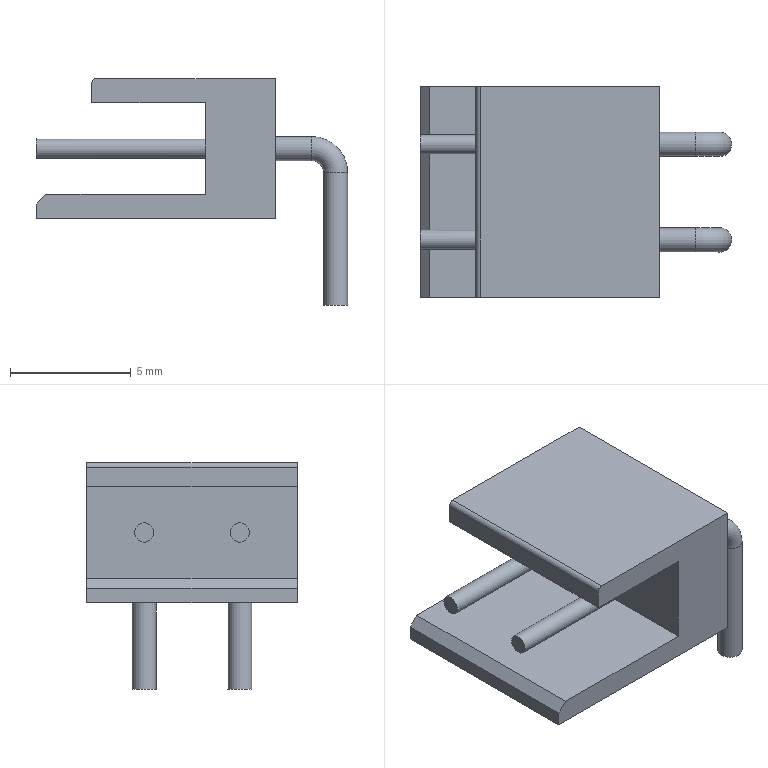Part | STEP file | JL27-02ZJW | 3 solids | 26 faces | box 12.9 x 8.72 x 9.401 mm | volume 271.213 mm3 | plane 17 | cylinder 7 | torus 2 | commonest cylinder face diameters 1 x4 0.795 x2 0.4 x1
STEP:
#1=CARTESIAN_POINT('',(0.,0.,0.));
#2=DIRECTION('',(0.,0.,1.));
#3=DIRECTION('',(1.,0.,0.));
#4=AXIS2_PLACEMENT_3D('',#1,#2,#3);
#5=CARTESIAN_POINT('',(-9.9,-2.377,0.));
#6=VERTEX_POINT('',#5);
#7=CARTESIAN_POINT('',(-9.9,-1.98,0.));
#8=DIRECTION('',(-1.,0.,0.));
#9=DIRECTION('',(0.,-1.,0.));
#10=AXIS2_PLACEMENT_3D('',#7,#8,#9);
#11=CIRCLE('',#10,0.3975);
#12=CARTESIAN_POINT('',(-9.9,-1.98,0.));
#13=DIRECTION('',(1.,0.,0.));
#14=DIRECTION('',(0.,0.,-1.));
#15=AXIS2_PLACEMENT_3D('',#12,#13,#14);
#16=CYLINDRICAL_SURFACE('',#15,0.3975);
#17=CARTESIAN_POINT('',(10.996,0.));
#18=DIRECTION('',(-1.,0.));
#19=VECTOR('',#18,1.);
#20=LINE('',#17,#19);
#21=(GEOMETRIC_REPRESENTATION_CONTEXT(2)PARAMETRIC_REPRESENTATION_CONTEXT()REPRESENTATION_CONTEXT('',''));
#22=DEFINITIONAL_REPRESENTATION('',(#20),#21);
#23=PCURVE('',#16,#22);
#24=CARTESIAN_POINT('',(-9.9,-1.98,0.));
#25=DIRECTION('',(-1.,0.,0.));
#26=DIRECTION('',(0.,0.,1.));
#27=AXIS2_PLACEMENT_3D('',#24,#25,#26);
#28=PLANE('',#27);
#29=CARTESIAN_POINT('',(0.,0.));
#30=DIRECTION('',(0.,-1.));
#31=AXIS2_PLACEMENT_2D('',#29,#30);
#32=CIRCLE('',#31,0.3975);
#33=(GEOMETRIC_REPRESENTATION_CONTEXT(2)PARAMETRIC_REPRESENTATION_CONTEXT()REPRESENTATION_CONTEXT('',''));
#34=DEFINITIONAL_REPRESENTATION('',(#32),#33);
#35=PCURVE('',#28,#34);
#36=SURFACE_CURVE('',#11,(#23,#35),.PCURVE_S1.);
#37=EDGE_CURVE('',#6,#6,#36,.T.);
#38=ORIENTED_EDGE('',*,*,#37,.F.);
#39=CARTESIAN_POINT('',(0.,-2.377,0.));
#40=VERTEX_POINT('',#39);
#41=CARTESIAN_POINT('',(-9.9,-2.377,0.));
#42=CARTESIAN_POINT('',(0.,-2.377,0.));
#43=B_SPLINE_CURVE_WITH_KNOTS('',1,(#41,#42),.UNSPECIFIED.,.F.,.F.,(2,2),(0.,9.9),.PIECEWISE_BEZIER_KNOTS.);
#44=CARTESIAN_POINT('',(10.996,0.));
#45=DIRECTION('',(0.,1.));
#46=VECTOR('',#45,1.);
#47=LINE('',#44,#46);
#48=(GEOMETRIC_REPRESENTATION_CONTEXT(2)PARAMETRIC_REPRESENTATION_CONTEXT()REPRESENTATION_CONTEXT('',''));
#49=DEFINITIONAL_REPRESENTATION('',(#47),#48);
#50=PCURVE('',#16,#49);
#51=CARTESIAN_POINT('',(4.712,0.));
#52=DIRECTION('',(0.,1.));
#53=VECTOR('',#52,1.);
#54=LINE('',#51,#53);
#55=(GEOMETRIC_REPRESENTATION_CONTEXT(2)PARAMETRIC_REPRESENTATION_CONTEXT()REPRESENTATION_CONTEXT('',''));
#56=DEFINITIONAL_REPRESENTATION('',(#54),#55);
#57=PCURVE('',#16,#56);
#58=SEAM_CURVE('',#43,(#50,#57),.PCURVE_S1.);
#59=EDGE_CURVE('',#6,#40,#58,.T.);
#60=ORIENTED_EDGE('',*,*,#59,.T.);
#61=CARTESIAN_POINT('',(0.,-1.98,0.3975));
#62=VERTEX_POINT('',#61);
#63=CARTESIAN_POINT('',(0.,-1.98,0.));
#64=DIRECTION('',(-1.,0.,0.));
#65=DIRECTION('',(0.,0.,1.));
#66=AXIS2_PLACEMENT_3D('',#63,#64,#65);
#67=CIRCLE('',#66,0.3975);
#68=CARTESIAN_POINT('',(15.708,9.9));
#69=DIRECTION('',(-1.,0.));
#70=VECTOR('',#69,1.);
#71=LINE('',#68,#70);
#72=(GEOMETRIC_REPRESENTATION_CONTEXT(2)PARAMETRIC_REPRESENTATION_CONTEXT()REPRESENTATION_CONTEXT('',''));
#73=DEFINITIONAL_REPRESENTATION('',(#71),#72);
#74=PCURVE('',#16,#73);
#75=CARTESIAN_POINT('',(0.,-1.98,-0.001008));
#76=DIRECTION('',(-1.,0.,0.));
#77=DIRECTION('',(0.,0.,1.));
#78=AXIS2_PLACEMENT_3D('',#75,#76,#77);
#79=PLANE('',#78);
#80=CARTESIAN_POINT('',(0.001008,0.));
#81=DIRECTION('',(1.,0.));
#82=AXIS2_PLACEMENT_2D('',#80,#81);
#83=CIRCLE('',#82,0.3975);
#84=(GEOMETRIC_REPRESENTATION_CONTEXT(2)PARAMETRIC_REPRESENTATION_CONTEXT()REPRESENTATION_CONTEXT('',''));
#85=DEFINITIONAL_REPRESENTATION('',(#83),#84);
#86=PCURVE('',#79,#85);
#87=SURFACE_CURVE('',#67,(#74,#86),.PCURVE_S1.);
#88=EDGE_CURVE('',#40,#62,#87,.T.);
#89=ORIENTED_EDGE('',*,*,#88,.T.);
#90=CARTESIAN_POINT('',(0.,-1.98,0.));
#91=DIRECTION('',(-1.,0.,0.));
#92=DIRECTION('',(0.,0.,1.));
#93=AXIS2_PLACEMENT_3D('',#90,#91,#92);
#94=CIRCLE('',#93,0.3975);
#95=CARTESIAN_POINT('',(9.425,9.9));
#96=DIRECTION('',(-1.,0.));
#97=VECTOR('',#96,1.);
#98=LINE('',#95,#97);
#99=(GEOMETRIC_REPRESENTATION_CONTEXT(2)PARAMETRIC_REPRESENTATION_CONTEXT()REPRESENTATION_CONTEXT('',''));
#100=DEFINITIONAL_REPRESENTATION('',(#98),#99);
#101=PCURVE('',#16,#100);
#102=CARTESIAN_POINT('',(0.001008,0.));
#103=DIRECTION('',(1.,0.));
#104=AXIS2_PLACEMENT_2D('',#102,#103);
#105=CIRCLE('',#104,0.3975);
#106=(GEOMETRIC_REPRESENTATION_CONTEXT(2)PARAMETRIC_REPRESENTATION_CONTEXT()REPRESENTATION_CONTEXT('',''));
#107=DEFINITIONAL_REPRESENTATION('',(#105),#106);
#108=PCURVE('',#79,#107);
#109=SURFACE_CURVE('',#94,(#101,#108),.PCURVE_S1.);
#110=EDGE_CURVE('',#62,#40,#109,.T.);
#111=ORIENTED_EDGE('',*,*,#110,.T.);
#112=ORIENTED_EDGE('',*,*,#59,.F.);
#113=EDGE_LOOP('',(#38,#60,#89,#111,#112));
#114=FACE_BOUND('',#113,.T.);
#115=ADVANCED_FACE('',(#114),#16,.T.);
#116=ORIENTED_EDGE('',*,*,#37,.T.);
#117=EDGE_LOOP('',(#116));
#118=FACE_BOUND('',#117,.T.);
#119=ADVANCED_FACE('',(#118),#28,.T.);
#120=CARTESIAN_POINT('',(0.,-1.98,0.499));
#121=VERTEX_POINT('',#120);
#122=CARTESIAN_POINT('',(0.,-1.98,-0.001008));
#123=DIRECTION('',(-1.,0.,0.));
#124=DIRECTION('',(0.,0.,1.));
#125=AXIS2_PLACEMENT_3D('',#122,#123,#124);
#126=CIRCLE('',#125,0.5);
#127=CARTESIAN_POINT('',(0.,0.));
#128=DIRECTION('',(1.,0.));
#129=AXIS2_PLACEMENT_2D('',#127,#128);
#130=CIRCLE('',#129,0.5);
#131=(GEOMETRIC_REPRESENTATION_CONTEXT(2)PARAMETRIC_REPRESENTATION_CONTEXT()REPRESENTATION_CONTEXT('',''));
#132=DEFINITIONAL_REPRESENTATION('',(#130),#131);
#133=PCURVE('',#79,#132);
#134=CARTESIAN_POINT('',(1.5,-1.98,-0.001008));
#135=DIRECTION('',(-1.,0.,0.));
#136=DIRECTION('',(0.,0.,1.));
#137=AXIS2_PLACEMENT_3D('',#134,#135,#136);
#138=CYLINDRICAL_SURFACE('',#137,0.5);
#139=CARTESIAN_POINT('',(0.,1.5));
#140=DIRECTION('',(1.,0.));
#141=VECTOR('',#140,1.);
#142=LINE('',#139,#141);
#143=(GEOMETRIC_REPRESENTATION_CONTEXT(2)PARAMETRIC_REPRESENTATION_CONTEXT()REPRESENTATION_CONTEXT('',''));
#144=DEFINITIONAL_REPRESENTATION('',(#142),#143);
#145=PCURVE('',#138,#144);
#146=SURFACE_CURVE('',#126,(#133,#145),.PCURVE_S1.);
#147=EDGE_CURVE('',#121,#121,#146,.T.);
#148=ORIENTED_EDGE('',*,*,#147,.T.);
#149=EDGE_LOOP('',(#148));
#150=FACE_BOUND('',#149,.T.);
#151=ORIENTED_EDGE('',*,*,#110,.F.);
#152=ORIENTED_EDGE('',*,*,#88,.F.);
#153=EDGE_LOOP('',(#151,#152));
#154=FACE_BOUND('',#153,.T.);
#155=ADVANCED_FACE('',(#150,#154),#79,.T.);
#156=CARTESIAN_POINT('',(1.5,-1.98,0.499));
#157=VERTEX_POINT('',#156);
#158=CARTESIAN_POINT('',(1.5,-1.98,-0.001008));
#159=DIRECTION('',(-1.,0.,0.));
#160=DIRECTION('',(0.,0.,1.));
#161=AXIS2_PLACEMENT_3D('',#158,#159,#160);
#162=CIRCLE('',#161,0.5);
#163=CARTESIAN_POINT('',(0.,0.));
#164=DIRECTION('',(1.,0.));
#165=VECTOR('',#164,1.);
#166=LINE('',#163,#165);
#167=(GEOMETRIC_REPRESENTATION_CONTEXT(2)PARAMETRIC_REPRESENTATION_CONTEXT()REPRESENTATION_CONTEXT('',''));
#168=DEFINITIONAL_REPRESENTATION('',(#166),#167);
#169=PCURVE('',#138,#168);
#170=CARTESIAN_POINT('',(1.5,-1.98,-1.001));
#171=DIRECTION('',(0.,-1.,0.));
#172=DIRECTION('',(0.,0.,-1.));
#173=AXIS2_PLACEMENT_3D('',#170,#171,#172);
#174=TOROIDAL_SURFACE('',#173,1.,0.5);
#175=CARTESIAN_POINT('',(9.425,6.283));
#176=DIRECTION('',(0.,-1.));
#177=VECTOR('',#176,1.);
#178=LINE('',#175,#177);
#179=(GEOMETRIC_REPRESENTATION_CONTEXT(2)PARAMETRIC_REPRESENTATION_CONTEXT()REPRESENTATION_CONTEXT('',''));
#180=DEFINITIONAL_REPRESENTATION('',(#178),#179);
#181=PCURVE('',#174,#180);
#182=SURFACE_CURVE('',#162,(#169,#181),.PCURVE_S1.);
#183=EDGE_CURVE('',#157,#157,#182,.T.);
#184=ORIENTED_EDGE('',*,*,#183,.T.);
#185=CARTESIAN_POINT('',(1.5,-1.98,0.499));
#186=CARTESIAN_POINT('',(0.,-1.98,0.499));
#187=B_SPLINE_CURVE_WITH_KNOTS('',1,(#185,#186),.UNSPECIFIED.,.F.,.F.,(2,2),(0.,1.5),.PIECEWISE_BEZIER_KNOTS.);
#188=CARTESIAN_POINT('',(6.283,0.));
#189=DIRECTION('',(0.,1.));
#190=VECTOR('',#189,1.);
#191=LINE('',#188,#190);
#192=(GEOMETRIC_REPRESENTATION_CONTEXT(2)PARAMETRIC_REPRESENTATION_CONTEXT()REPRESENTATION_CONTEXT('',''));
#193=DEFINITIONAL_REPRESENTATION('',(#191),#192);
#194=PCURVE('',#138,#193);
#195=CARTESIAN_POINT('',(0.,0.));
#196=DIRECTION('',(0.,1.));
#197=VECTOR('',#196,1.);
#198=LINE('',#195,#197);
#199=(GEOMETRIC_REPRESENTATION_CONTEXT(2)PARAMETRIC_REPRESENTATION_CONTEXT()REPRESENTATION_CONTEXT('',''));
#200=DEFINITIONAL_REPRESENTATION('',(#198),#199);
#201=PCURVE('',#138,#200);
#202=SEAM_CURVE('',#187,(#194,#201),.PCURVE_S1.);
#203=EDGE_CURVE('',#157,#121,#202,.T.);
#204=ORIENTED_EDGE('',*,*,#203,.T.);
#205=ORIENTED_EDGE('',*,*,#147,.F.);
#206=ORIENTED_EDGE('',*,*,#203,.F.);
#207=EDGE_LOOP('',(#184,#204,#205,#206));
#208=FACE_BOUND('',#207,.T.);
#209=ADVANCED_FACE('',(#208),#138,.T.);
#210=CARTESIAN_POINT('',(3.,-1.98,-1.001));
#211=VERTEX_POINT('',#210);
#212=CARTESIAN_POINT('',(2.5,-1.98,-1.001));
#213=DIRECTION('',(0.,0.,1.));
#214=DIRECTION('',(1.,0.,0.));
#215=AXIS2_PLACEMENT_3D('',#212,#213,#214);
#216=CIRCLE('',#215,0.5);
#217=CARTESIAN_POINT('',(7.854,6.283));
#218=DIRECTION('',(0.,-1.));
#219=VECTOR('',#218,1.);
#220=LINE('',#217,#219);
#221=(GEOMETRIC_REPRESENTATION_CONTEXT(2)PARAMETRIC_REPRESENTATION_CONTEXT()REPRESENTATION_CONTEXT('',''));
#222=DEFINITIONAL_REPRESENTATION('',(#220),#221);
#223=PCURVE('',#174,#222);
#224=CARTESIAN_POINT('',(2.5,-1.98,-1.001));
#225=DIRECTION('',(0.,0.,-1.));
#226=DIRECTION('',(-1.,0.,0.));
#227=AXIS2_PLACEMENT_3D('',#224,#225,#226);
#228=CYLINDRICAL_SURFACE('',#227,0.5);
#229=CARTESIAN_POINT('',(9.425,0.));
#230=DIRECTION('',(-1.,0.));
#231=VECTOR('',#230,1.);
#232=LINE('',#229,#231);
#233=(GEOMETRIC_REPRESENTATION_CONTEXT(2)PARAMETRIC_REPRESENTATION_CONTEXT()REPRESENTATION_CONTEXT('',''));
#234=DEFINITIONAL_REPRESENTATION('',(#232),#233);
#235=PCURVE('',#228,#234);
#236=SURFACE_CURVE('',#216,(#223,#235),.PCURVE_S1.);
#237=EDGE_CURVE('',#211,#211,#236,.T.);
#238=ORIENTED_EDGE('',*,*,#237,.T.);
#239=CARTESIAN_POINT('',(3.,-1.98,-1.001));
#240=CARTESIAN_POINT('',(3.,-1.98,-0.6));
#241=CARTESIAN_POINT('',(2.872,-1.98,-0.2094));
#242=CARTESIAN_POINT('',(2.628,-1.98,0.1269));
#243=CARTESIAN_POINT('',(2.292,-1.98,0.3715));
#244=CARTESIAN_POINT('',(1.901,-1.98,0.499));
#245=CARTESIAN_POINT('',(1.5,-1.98,0.499));
#246=(BOUNDED_CURVE()B_SPLINE_CURVE(6,(#239,#240,#241,#242,#243,#244,#245),.UNSPECIFIED.,.F.,.F.)B_SPLINE_CURVE_WITH_KNOTS((7,7),(1.571,3.142),.PIECEWISE_BEZIER_KNOTS.)CURVE()GEOMETRIC_REPRESENTATION_ITEM()RATIONAL_B_SPLINE_CURVE((1.031,1.01,0.9979,0.994,0.9979,1.01,1.031))REPRESENTATION_ITEM(''));
#247=CARTESIAN_POINT('',(6.283,0.));
#248=DIRECTION('',(1.,0.));
#249=VECTOR('',#248,1.);
#250=LINE('',#247,#249);
#251=(GEOMETRIC_REPRESENTATION_CONTEXT(2)PARAMETRIC_REPRESENTATION_CONTEXT()REPRESENTATION_CONTEXT('',''));
#252=DEFINITIONAL_REPRESENTATION('',(#250),#251);
#253=PCURVE('',#174,#252);
#254=CARTESIAN_POINT('',(6.283,6.283));
#255=DIRECTION('',(1.,0.));
#256=VECTOR('',#255,1.);
#257=LINE('',#254,#256);
#258=(GEOMETRIC_REPRESENTATION_CONTEXT(2)PARAMETRIC_REPRESENTATION_CONTEXT()REPRESENTATION_CONTEXT('',''));
#259=DEFINITIONAL_REPRESENTATION('',(#257),#258);
#260=PCURVE('',#174,#259);
#261=SEAM_CURVE('',#246,(#253,#260),.PCURVE_S1.);
#262=EDGE_CURVE('',#211,#157,#261,.T.);
#263=ORIENTED_EDGE('',*,*,#262,.T.);
#264=ORIENTED_EDGE('',*,*,#183,.F.);
#265=ORIENTED_EDGE('',*,*,#262,.F.);
#266=EDGE_LOOP('',(#238,#263,#264,#265));
#267=FACE_BOUND('',#266,.T.);
#268=ADVANCED_FACE('',(#267),#174,.T.);
#269=ORIENTED_EDGE('',*,*,#237,.F.);
#270=CARTESIAN_POINT('',(3.,-1.98,-6.501));
#271=VERTEX_POINT('',#270);
#272=CARTESIAN_POINT('',(3.,-1.98,-1.001));
#273=CARTESIAN_POINT('',(3.,-1.98,-6.501));
#274=B_SPLINE_CURVE_WITH_KNOTS('',1,(#272,#273),.UNSPECIFIED.,.F.,.F.,(2,2),(0.,5.5),.PIECEWISE_BEZIER_KNOTS.);
#275=CARTESIAN_POINT('',(9.425,0.));
#276=DIRECTION('',(0.,1.));
#277=VECTOR('',#276,1.);
#278=LINE('',#275,#277);
#279=(GEOMETRIC_REPRESENTATION_CONTEXT(2)PARAMETRIC_REPRESENTATION_CONTEXT()REPRESENTATION_CONTEXT('',''));
#280=DEFINITIONAL_REPRESENTATION('',(#278),#279);
#281=PCURVE('',#228,#280);
#282=CARTESIAN_POINT('',(3.142,0.));
#283=DIRECTION('',(0.,1.));
#284=VECTOR('',#283,1.);
#285=LINE('',#282,#284);
#286=(GEOMETRIC_REPRESENTATION_CONTEXT(2)PARAMETRIC_REPRESENTATION_CONTEXT()REPRESENTATION_CONTEXT('',''));
#287=DEFINITIONAL_REPRESENTATION('',(#285),#286);
#288=PCURVE('',#228,#287);
#289=SEAM_CURVE('',#274,(#281,#288),.PCURVE_S1.);
#290=EDGE_CURVE('',#211,#271,#289,.T.);
#291=ORIENTED_EDGE('',*,*,#290,.T.);
#292=CARTESIAN_POINT('',(2.5,-1.98,-6.501));
#293=DIRECTION('',(0.,0.,1.));
#294=DIRECTION('',(1.,0.,0.));
#295=AXIS2_PLACEMENT_3D('',#292,#293,#294);
#296=CIRCLE('',#295,0.5);
#297=CARTESIAN_POINT('',(9.425,5.5));
#298=DIRECTION('',(-1.,0.));
#299=VECTOR('',#298,1.);
#300=LINE('',#297,#299);
#301=(GEOMETRIC_REPRESENTATION_CONTEXT(2)PARAMETRIC_REPRESENTATION_CONTEXT()REPRESENTATION_CONTEXT('',''));
#302=DEFINITIONAL_REPRESENTATION('',(#300),#301);
#303=PCURVE('',#228,#302);
#304=CARTESIAN_POINT('',(2.5,-1.98,-6.501));
#305=DIRECTION('',(0.,0.,1.));
#306=DIRECTION('',(1.,0.,0.));
#307=AXIS2_PLACEMENT_3D('',#304,#305,#306);
#308=PLANE('',#307);
#309=CARTESIAN_POINT('',(0.,0.));
#310=DIRECTION('',(1.,0.));
#311=AXIS2_PLACEMENT_2D('',#309,#310);
#312=CIRCLE('',#311,0.5);
#313=(GEOMETRIC_REPRESENTATION_CONTEXT(2)PARAMETRIC_REPRESENTATION_CONTEXT()REPRESENTATION_CONTEXT('',''));
#314=DEFINITIONAL_REPRESENTATION('',(#312),#313);
#315=PCURVE('',#308,#314);
#316=SURFACE_CURVE('',#296,(#303,#315),.PCURVE_S1.);
#317=EDGE_CURVE('',#271,#271,#316,.T.);
#318=ORIENTED_EDGE('',*,*,#317,.T.);
#319=ORIENTED_EDGE('',*,*,#290,.F.);
#320=EDGE_LOOP('',(#269,#291,#318,#319));
#321=FACE_BOUND('',#320,.T.);
#322=ADVANCED_FACE('',(#321),#228,.T.);
#323=ORIENTED_EDGE('',*,*,#317,.F.);
#324=EDGE_LOOP('',(#323));
#325=FACE_BOUND('',#324,.T.);
#326=ADVANCED_FACE('',(#325),#308,.F.);
#327=CLOSED_SHELL('',(#115,#119,#155,#209,#268,#322,#326));
#328=MANIFOLD_SOLID_BREP('',#327);
#329=CARTESIAN_POINT('',(-2.9,4.36,1.9));
#330=VERTEX_POINT('',#329);
#331=CARTESIAN_POINT('',(-2.9,-4.36,1.9));
#332=VERTEX_POINT('',#331);
#333=CARTESIAN_POINT('',(-2.9,4.36,1.9));
#334=DIRECTION('',(0.,-1.,0.));
#335=VECTOR('',#334,1.);
#336=LINE('',#333,#335);
#337=CARTESIAN_POINT('',(-2.9,0.,0.));
#338=DIRECTION('',(1.,0.,0.));
#339=DIRECTION('',(0.,0.,-1.));
#340=AXIS2_PLACEMENT_3D('',#337,#338,#339);
#341=PLANE('',#340);
#342=CARTESIAN_POINT('',(-1.9,4.36));
#343=DIRECTION('',(0.,-1.));
#344=VECTOR('',#343,1.);
#345=LINE('',#342,#344);
#346=(GEOMETRIC_REPRESENTATION_CONTEXT(2)PARAMETRIC_REPRESENTATION_CONTEXT()REPRESENTATION_CONTEXT('',''));
#347=DEFINITIONAL_REPRESENTATION('',(#345),#346);
#348=PCURVE('',#341,#347);
#349=CARTESIAN_POINT('',(-7.6,4.36,1.9));
#350=DIRECTION('',(0.,0.,1.));
#351=DIRECTION('',(1.,0.,0.));
#352=AXIS2_PLACEMENT_3D('',#349,#350,#351);
#353=PLANE('',#352);
#354=CARTESIAN_POINT('',(4.7,0.));
#355=DIRECTION('',(0.,-1.));
#356=VECTOR('',#355,1.);
#357=LINE('',#354,#356);
#358=(GEOMETRIC_REPRESENTATION_CONTEXT(2)PARAMETRIC_REPRESENTATION_CONTEXT()REPRESENTATION_CONTEXT('',''));
#359=DEFINITIONAL_REPRESENTATION('',(#357),#358);
#360=PCURVE('',#353,#359);
#361=SURFACE_CURVE('',#336,(#348,#360),.PCURVE_S1.);
#362=EDGE_CURVE('',#330,#332,#361,.T.);
#363=ORIENTED_EDGE('',*,*,#362,.F.);
#364=CARTESIAN_POINT('',(-2.9,4.36,-1.9));
#365=VERTEX_POINT('',#364);
#366=CARTESIAN_POINT('',(-2.9,4.36,-2.9));
#367=DIRECTION('',(0.,0.,-1.));
#368=VECTOR('',#367,1.);
#369=LINE('',#366,#368);
#370=CARTESIAN_POINT('',(2.9,4.36));
#371=DIRECTION('',(1.,0.));
#372=VECTOR('',#371,1.);
#373=LINE('',#370,#372);
#374=(GEOMETRIC_REPRESENTATION_CONTEXT(2)PARAMETRIC_REPRESENTATION_CONTEXT()REPRESENTATION_CONTEXT('',''));
#375=DEFINITIONAL_REPRESENTATION('',(#373),#374);
#376=PCURVE('',#341,#375);
#377=CARTESIAN_POINT('',(-2.9,4.36,-2.9));
#378=DIRECTION('',(0.,1.,0.));
#379=DIRECTION('',(0.,0.,1.));
#380=AXIS2_PLACEMENT_3D('',#377,#378,#379);
#381=PLANE('',#380);
#382=CARTESIAN_POINT('',(0.,0.));
#383=DIRECTION('',(-1.,0.));
#384=VECTOR('',#383,1.);
#385=LINE('',#382,#384);
#386=(GEOMETRIC_REPRESENTATION_CONTEXT(2)PARAMETRIC_REPRESENTATION_CONTEXT()REPRESENTATION_CONTEXT('',''));
#387=DEFINITIONAL_REPRESENTATION('',(#385),#386);
#388=PCURVE('',#381,#387);
#389=SURFACE_CURVE('',#369,(#376,#388),.PCURVE_S1.);
#390=EDGE_CURVE('',#330,#365,#389,.T.);
#391=ORIENTED_EDGE('',*,*,#390,.T.);
#392=CARTESIAN_POINT('',(-2.9,-4.36,-1.9));
#393=VERTEX_POINT('',#392);
#394=CARTESIAN_POINT('',(-2.9,-4.36,-1.9));
#395=DIRECTION('',(0.,1.,0.));
#396=VECTOR('',#395,1.);
#397=LINE('',#394,#396);
#398=CARTESIAN_POINT('',(1.9,-4.36));
#399=DIRECTION('',(0.,1.));
#400=VECTOR('',#399,1.);
#401=LINE('',#398,#400);
#402=(GEOMETRIC_REPRESENTATION_CONTEXT(2)PARAMETRIC_REPRESENTATION_CONTEXT()REPRESENTATION_CONTEXT('',''));
#403=DEFINITIONAL_REPRESENTATION('',(#401),#402);
#404=PCURVE('',#341,#403);
#405=CARTESIAN_POINT('',(-9.9,-4.36,-1.9));
#406=DIRECTION('',(0.,0.,-1.));
#407=DIRECTION('',(0.,1.,0.));
#408=AXIS2_PLACEMENT_3D('',#405,#406,#407);
#409=PLANE('',#408);
#410=CARTESIAN_POINT('',(0.,7.));
#411=DIRECTION('',(1.,0.));
#412=VECTOR('',#411,1.);
#413=LINE('',#410,#412);
#414=(GEOMETRIC_REPRESENTATION_CONTEXT(2)PARAMETRIC_REPRESENTATION_CONTEXT()REPRESENTATION_CONTEXT('',''));
#415=DEFINITIONAL_REPRESENTATION('',(#413),#414);
#416=PCURVE('',#409,#415);
#417=SURFACE_CURVE('',#397,(#404,#416),.PCURVE_S1.);
#418=EDGE_CURVE('',#393,#365,#417,.T.);
#419=ORIENTED_EDGE('',*,*,#418,.F.);
#420=CARTESIAN_POINT('',(-2.9,-4.36,2.9));
#421=DIRECTION('',(0.,0.,1.));
#422=VECTOR('',#421,1.);
#423=LINE('',#420,#422);
#424=CARTESIAN_POINT('',(-2.9,-4.36));
#425=DIRECTION('',(-1.,0.));
#426=VECTOR('',#425,1.);
#427=LINE('',#424,#426);
#428=(GEOMETRIC_REPRESENTATION_CONTEXT(2)PARAMETRIC_REPRESENTATION_CONTEXT()REPRESENTATION_CONTEXT('',''));
#429=DEFINITIONAL_REPRESENTATION('',(#427),#428);
#430=PCURVE('',#341,#429);
#431=CARTESIAN_POINT('',(-2.9,-4.36,2.9));
#432=DIRECTION('',(0.,-1.,0.));
#433=DIRECTION('',(0.,0.,-1.));
#434=AXIS2_PLACEMENT_3D('',#431,#432,#433);
#435=PLANE('',#434);
#436=CARTESIAN_POINT('',(0.,0.));
#437=DIRECTION('',(-1.,0.));
#438=VECTOR('',#437,1.);
#439=LINE('',#436,#438);
#440=(GEOMETRIC_REPRESENTATION_CONTEXT(2)PARAMETRIC_REPRESENTATION_CONTEXT()REPRESENTATION_CONTEXT('',''));
#441=DEFINITIONAL_REPRESENTATION('',(#439),#440);
#442=PCURVE('',#435,#441);
#443=SURFACE_CURVE('',#423,(#430,#442),.PCURVE_S1.);
#444=EDGE_CURVE('',#393,#332,#443,.T.);
#445=ORIENTED_EDGE('',*,*,#444,.T.);
#446=EDGE_LOOP('',(#363,#391,#419,#445));
#447=FACE_BOUND('',#446,.T.);
#448=ADVANCED_FACE('',(#447),#341,.F.);
#449=CARTESIAN_POINT('',(-9.5,-4.36,-1.9));
#450=VERTEX_POINT('',#449);
#451=CARTESIAN_POINT('',(-9.9,-4.36,-1.9));
#452=DIRECTION('',(1.,0.,0.));
#453=VECTOR('',#452,1.);
#454=LINE('',#451,#453);
#455=CARTESIAN_POINT('',(4.8,-7.));
#456=DIRECTION('',(0.,1.));
#457=VECTOR('',#456,1.);
#458=LINE('',#455,#457);
#459=(GEOMETRIC_REPRESENTATION_CONTEXT(2)PARAMETRIC_REPRESENTATION_CONTEXT()REPRESENTATION_CONTEXT('',''));
#460=DEFINITIONAL_REPRESENTATION('',(#458),#459);
#461=PCURVE('',#435,#460);
#462=CARTESIAN_POINT('',(0.,0.));
#463=DIRECTION('',(0.,1.));
#464=VECTOR('',#463,1.);
#465=LINE('',#462,#464);
#466=(GEOMETRIC_REPRESENTATION_CONTEXT(2)PARAMETRIC_REPRESENTATION_CONTEXT()REPRESENTATION_CONTEXT('',''));
#467=DEFINITIONAL_REPRESENTATION('',(#465),#466);
#468=PCURVE('',#409,#467);
#469=SURFACE_CURVE('',#454,(#461,#468),.PCURVE_S1.);
#470=EDGE_CURVE('',#450,#393,#469,.T.);
#471=ORIENTED_EDGE('',*,*,#470,.F.);
#472=CARTESIAN_POINT('',(-9.9,-4.36,-2.3));
#473=VERTEX_POINT('',#472);
#474=CARTESIAN_POINT('',(-3.8,-4.36,3.8));
#475=DIRECTION('',(-0.7071,0.,-0.7071));
#476=VECTOR('',#475,1.);
#477=LINE('',#474,#476);
#478=CARTESIAN_POINT('',(-0.9,-0.9));
#479=DIRECTION('',(0.7071,-0.7071));
#480=VECTOR('',#479,1.);
#481=LINE('',#478,#480);
#482=(GEOMETRIC_REPRESENTATION_CONTEXT(2)PARAMETRIC_REPRESENTATION_CONTEXT()REPRESENTATION_CONTEXT('',''));
#483=DEFINITIONAL_REPRESENTATION('',(#481),#482);
#484=PCURVE('',#435,#483);
#485=CARTESIAN_POINT('',(-9.9,0.,-2.3));
#486=DIRECTION('',(-0.7071,0.,0.7071));
#487=DIRECTION('',(0.,-1.,0.));
#488=AXIS2_PLACEMENT_3D('',#485,#486,#487);
#489=PLANE('',#488);
#490=CARTESIAN_POINT('',(4.36,8.627));
#491=DIRECTION('',(0.,-1.));
#492=VECTOR('',#491,1.);
#493=LINE('',#490,#492);
#494=(GEOMETRIC_REPRESENTATION_CONTEXT(2)PARAMETRIC_REPRESENTATION_CONTEXT()REPRESENTATION_CONTEXT('',''));
#495=DEFINITIONAL_REPRESENTATION('',(#493),#494);
#496=PCURVE('',#489,#495);
#497=SURFACE_CURVE('',#477,(#484,#496),.PCURVE_S1.);
#498=EDGE_CURVE('',#450,#473,#497,.T.);
#499=ORIENTED_EDGE('',*,*,#498,.T.);
#500=CARTESIAN_POINT('',(-9.9,-4.36,-2.9));
#501=VERTEX_POINT('',#500);
#502=CARTESIAN_POINT('',(-9.9,-4.36,-2.9));
#503=DIRECTION('',(0.,0.,1.));
#504=VECTOR('',#503,1.);
#505=LINE('',#502,#504);
#506=CARTESIAN_POINT('',(5.8,-7.));
#507=DIRECTION('',(-1.,0.));
#508=VECTOR('',#507,1.);
#509=LINE('',#506,#508);
#510=(GEOMETRIC_REPRESENTATION_CONTEXT(2)PARAMETRIC_REPRESENTATION_CONTEXT()REPRESENTATION_CONTEXT('',''));
#511=DEFINITIONAL_REPRESENTATION('',(#509),#510);
#512=PCURVE('',#435,#511);
#513=CARTESIAN_POINT('',(-9.9,0.,0.));
#514=DIRECTION('',(-1.,0.,0.));
#515=DIRECTION('',(0.,0.,1.));
#516=AXIS2_PLACEMENT_3D('',#513,#514,#515);
#517=PLANE('',#516);
#518=CARTESIAN_POINT('',(-2.9,-4.36));
#519=DIRECTION('',(1.,0.));
#520=VECTOR('',#519,1.);
#521=LINE('',#518,#520);
#522=(GEOMETRIC_REPRESENTATION_CONTEXT(2)PARAMETRIC_REPRESENTATION_CONTEXT()REPRESENTATION_CONTEXT('',''));
#523=DEFINITIONAL_REPRESENTATION('',(#521),#522);
#524=PCURVE('',#517,#523);
#525=SURFACE_CURVE('',#505,(#512,#524),.PCURVE_S1.);
#526=EDGE_CURVE('',#501,#473,#525,.T.);
#527=ORIENTED_EDGE('',*,*,#526,.F.);
#528=CARTESIAN_POINT('',(0.,-4.36,-2.9));
#529=VERTEX_POINT('',#528);
#530=CARTESIAN_POINT('',(-2.9,-4.36,-2.9));
#531=DIRECTION('',(-1.,0.,0.));
#532=VECTOR('',#531,1.);
#533=LINE('',#530,#532);
#534=CARTESIAN_POINT('',(5.8,0.));
#535=DIRECTION('',(0.,-1.));
#536=VECTOR('',#535,1.);
#537=LINE('',#534,#536);
#538=(GEOMETRIC_REPRESENTATION_CONTEXT(2)PARAMETRIC_REPRESENTATION_CONTEXT()REPRESENTATION_CONTEXT('',''));
#539=DEFINITIONAL_REPRESENTATION('',(#537),#538);
#540=PCURVE('',#435,#539);
#541=CARTESIAN_POINT('',(-2.9,-4.36,-2.9));
#542=DIRECTION('',(0.,0.,-1.));
#543=DIRECTION('',(-1.,0.,0.));
#544=AXIS2_PLACEMENT_3D('',#541,#542,#543);
#545=PLANE('',#544);
#546=CARTESIAN_POINT('',(0.,0.));
#547=DIRECTION('',(1.,0.));
#548=VECTOR('',#547,1.);
#549=LINE('',#546,#548);
#550=(GEOMETRIC_REPRESENTATION_CONTEXT(2)PARAMETRIC_REPRESENTATION_CONTEXT()REPRESENTATION_CONTEXT('',''));
#551=DEFINITIONAL_REPRESENTATION('',(#549),#550);
#552=PCURVE('',#545,#551);
#553=SURFACE_CURVE('',#533,(#540,#552),.PCURVE_S1.);
#554=EDGE_CURVE('',#529,#501,#553,.T.);
#555=ORIENTED_EDGE('',*,*,#554,.F.);
#556=CARTESIAN_POINT('',(0.,-4.36,2.9));
#557=VERTEX_POINT('',#556);
#558=CARTESIAN_POINT('',(0.,-4.36,2.9));
#559=DIRECTION('',(0.,0.,1.));
#560=VECTOR('',#559,1.);
#561=LINE('',#558,#560);
#562=CARTESIAN_POINT('',(0.,2.9));
#563=DIRECTION('',(-1.,0.));
#564=VECTOR('',#563,1.);
#565=LINE('',#562,#564);
#566=(GEOMETRIC_REPRESENTATION_CONTEXT(2)PARAMETRIC_REPRESENTATION_CONTEXT()REPRESENTATION_CONTEXT('',''));
#567=DEFINITIONAL_REPRESENTATION('',(#565),#566);
#568=PCURVE('',#435,#567);
#569=CARTESIAN_POINT('',(0.,0.,0.));
#570=DIRECTION('',(1.,0.,0.));
#571=DIRECTION('',(0.,0.,-1.));
#572=AXIS2_PLACEMENT_3D('',#569,#570,#571);
#573=PLANE('',#572);
#574=CARTESIAN_POINT('',(-2.9,-4.36));
#575=DIRECTION('',(-1.,0.));
#576=VECTOR('',#575,1.);
#577=LINE('',#574,#576);
#578=(GEOMETRIC_REPRESENTATION_CONTEXT(2)PARAMETRIC_REPRESENTATION_CONTEXT()REPRESENTATION_CONTEXT('',''));
#579=DEFINITIONAL_REPRESENTATION('',(#577),#578);
#580=PCURVE('',#573,#579);
#581=SURFACE_CURVE('',#561,(#568,#580),.PCURVE_S1.);
#582=EDGE_CURVE('',#529,#557,#581,.T.);
#583=ORIENTED_EDGE('',*,*,#582,.T.);
#584=CARTESIAN_POINT('',(-7.4,-4.36,2.9));
#585=VERTEX_POINT('',#584);
#586=CARTESIAN_POINT('',(-2.9,-4.36,2.9));
#587=DIRECTION('',(-1.,0.,0.));
#588=VECTOR('',#587,1.);
#589=LINE('',#586,#588);
#590=CARTESIAN_POINT('',(0.,0.));
#591=DIRECTION('',(0.,-1.));
#592=VECTOR('',#591,1.);
#593=LINE('',#590,#592);
#594=(GEOMETRIC_REPRESENTATION_CONTEXT(2)PARAMETRIC_REPRESENTATION_CONTEXT()REPRESENTATION_CONTEXT('',''));
#595=DEFINITIONAL_REPRESENTATION('',(#593),#594);
#596=PCURVE('',#435,#595);
#597=CARTESIAN_POINT('',(-2.9,4.36,2.9));
#598=DIRECTION('',(0.,0.,1.));
#599=DIRECTION('',(1.,0.,0.));
#600=AXIS2_PLACEMENT_3D('',#597,#598,#599);
#601=PLANE('',#600);
#602=CARTESIAN_POINT('',(0.,-8.72));
#603=DIRECTION('',(-1.,0.));
#604=VECTOR('',#603,1.);
#605=LINE('',#602,#604);
#606=(GEOMETRIC_REPRESENTATION_CONTEXT(2)PARAMETRIC_REPRESENTATION_CONTEXT()REPRESENTATION_CONTEXT('',''));
#607=DEFINITIONAL_REPRESENTATION('',(#605),#606);
#608=PCURVE('',#601,#607);
#609=SURFACE_CURVE('',#589,(#596,#608),.PCURVE_S1.);
#610=EDGE_CURVE('',#557,#585,#609,.T.);
#611=ORIENTED_EDGE('',*,*,#610,.T.);
#612=CARTESIAN_POINT('',(-7.6,-4.36,2.7));
#613=VERTEX_POINT('',#612);
#614=CARTESIAN_POINT('',(-7.4,-4.36,2.7));
#615=DIRECTION('',(0.,-1.,0.));
#616=DIRECTION('',(0.,0.,-1.));
#617=AXIS2_PLACEMENT_3D('',#614,#615,#616);
#618=CIRCLE('',#617,0.2);
#619=CARTESIAN_POINT('',(0.2,-4.5));
#620=DIRECTION('',(1.,0.));
#621=AXIS2_PLACEMENT_2D('',#619,#620);
#622=CIRCLE('',#621,0.2);
#623=(GEOMETRIC_REPRESENTATION_CONTEXT(2)PARAMETRIC_REPRESENTATION_CONTEXT()REPRESENTATION_CONTEXT('',''));
#624=DEFINITIONAL_REPRESENTATION('',(#622),#623);
#625=PCURVE('',#435,#624);
#626=CARTESIAN_POINT('',(-7.4,0.,2.7));
#627=DIRECTION('',(0.,1.,0.));
#628=DIRECTION('',(0.,0.,1.));
#629=AXIS2_PLACEMENT_3D('',#626,#627,#628);
#630=CYLINDRICAL_SURFACE('',#629,0.2);
#631=CARTESIAN_POINT('',(9.425,-4.36));
#632=DIRECTION('',(-1.,0.));
#633=VECTOR('',#632,1.);
#634=LINE('',#631,#633);
#635=(GEOMETRIC_REPRESENTATION_CONTEXT(2)PARAMETRIC_REPRESENTATION_CONTEXT()REPRESENTATION_CONTEXT('',''));
#636=DEFINITIONAL_REPRESENTATION('',(#634),#635);
#637=PCURVE('',#630,#636);
#638=SURFACE_CURVE('',#618,(#625,#637),.PCURVE_S1.);
#639=EDGE_CURVE('',#585,#613,#638,.T.);
#640=ORIENTED_EDGE('',*,*,#639,.T.);
#641=CARTESIAN_POINT('',(-7.6,-4.36,1.9));
#642=VERTEX_POINT('',#641);
#643=CARTESIAN_POINT('',(-7.6,-4.36,1.9));
#644=DIRECTION('',(0.,0.,1.));
#645=VECTOR('',#644,1.);
#646=LINE('',#643,#645);
#647=CARTESIAN_POINT('',(1.,-4.7));
#648=DIRECTION('',(-1.,0.));
#649=VECTOR('',#648,1.);
#650=LINE('',#647,#649);
#651=(GEOMETRIC_REPRESENTATION_CONTEXT(2)PARAMETRIC_REPRESENTATION_CONTEXT()REPRESENTATION_CONTEXT('',''));
#652=DEFINITIONAL_REPRESENTATION('',(#650),#651);
#653=PCURVE('',#435,#652);
#654=CARTESIAN_POINT('',(-7.6,0.,0.));
#655=DIRECTION('',(-1.,0.,0.));
#656=DIRECTION('',(0.,0.,1.));
#657=AXIS2_PLACEMENT_3D('',#654,#655,#656);
#658=PLANE('',#657);
#659=CARTESIAN_POINT('',(1.9,-4.36));
#660=DIRECTION('',(1.,0.));
#661=VECTOR('',#660,1.);
#662=LINE('',#659,#661);
#663=(GEOMETRIC_REPRESENTATION_CONTEXT(2)PARAMETRIC_REPRESENTATION_CONTEXT()REPRESENTATION_CONTEXT('',''));
#664=DEFINITIONAL_REPRESENTATION('',(#662),#663);
#665=PCURVE('',#658,#664);
#666=SURFACE_CURVE('',#646,(#653,#665),.PCURVE_S1.);
#667=EDGE_CURVE('',#642,#613,#666,.T.);
#668=ORIENTED_EDGE('',*,*,#667,.F.);
#669=CARTESIAN_POINT('',(-7.6,-4.36,1.9));
#670=DIRECTION('',(1.,0.,0.));
#671=VECTOR('',#670,1.);
#672=LINE('',#669,#671);
#673=CARTESIAN_POINT('',(1.,-4.7));
#674=DIRECTION('',(0.,1.));
#675=VECTOR('',#674,1.);
#676=LINE('',#673,#675);
#677=(GEOMETRIC_REPRESENTATION_CONTEXT(2)PARAMETRIC_REPRESENTATION_CONTEXT()REPRESENTATION_CONTEXT('',''));
#678=DEFINITIONAL_REPRESENTATION('',(#676),#677);
#679=PCURVE('',#435,#678);
#680=CARTESIAN_POINT('',(0.,-8.72));
#681=DIRECTION('',(1.,0.));
#682=VECTOR('',#681,1.);
#683=LINE('',#680,#682);
#684=(GEOMETRIC_REPRESENTATION_CONTEXT(2)PARAMETRIC_REPRESENTATION_CONTEXT()REPRESENTATION_CONTEXT('',''));
#685=DEFINITIONAL_REPRESENTATION('',(#683),#684);
#686=PCURVE('',#353,#685);
#687=SURFACE_CURVE('',#672,(#679,#686),.PCURVE_S1.);
#688=EDGE_CURVE('',#642,#332,#687,.T.);
#689=ORIENTED_EDGE('',*,*,#688,.T.);
#690=ORIENTED_EDGE('',*,*,#444,.F.);
#691=EDGE_LOOP('',(#471,#499,#527,#555,#583,#611,#640,#668,#689,#690));
#692=FACE_BOUND('',#691,.T.);
#693=ADVANCED_FACE('',(#692),#435,.T.);
#694=CARTESIAN_POINT('',(0.,4.36,-2.9));
#695=VERTEX_POINT('',#694);
#696=CARTESIAN_POINT('',(0.,-4.36,-2.9));
#697=DIRECTION('',(0.,-1.,0.));
#698=VECTOR('',#697,1.);
#699=LINE('',#696,#698);
#700=CARTESIAN_POINT('',(-2.9,0.));
#701=DIRECTION('',(0.,-1.));
#702=VECTOR('',#701,1.);
#703=LINE('',#700,#702);
#704=(GEOMETRIC_REPRESENTATION_CONTEXT(2)PARAMETRIC_REPRESENTATION_CONTEXT()REPRESENTATION_CONTEXT('',''));
#705=DEFINITIONAL_REPRESENTATION('',(#703),#704);
#706=PCURVE('',#545,#705);
#707=CARTESIAN_POINT('',(2.9,-4.36));
#708=DIRECTION('',(0.,-1.));
#709=VECTOR('',#708,1.);
#710=LINE('',#707,#709);
#711=(GEOMETRIC_REPRESENTATION_CONTEXT(2)PARAMETRIC_REPRESENTATION_CONTEXT()REPRESENTATION_CONTEXT('',''));
#712=DEFINITIONAL_REPRESENTATION('',(#710),#711);
#713=PCURVE('',#573,#712);
#714=SURFACE_CURVE('',#699,(#706,#713),.PCURVE_S1.);
#715=EDGE_CURVE('',#695,#529,#714,.T.);
#716=ORIENTED_EDGE('',*,*,#715,.T.);
#717=ORIENTED_EDGE('',*,*,#554,.T.);
#718=CARTESIAN_POINT('',(-9.9,4.36,-2.9));
#719=VERTEX_POINT('',#718);
#720=CARTESIAN_POINT('',(-9.9,4.36,-2.9));
#721=DIRECTION('',(0.,-1.,0.));
#722=VECTOR('',#721,1.);
#723=LINE('',#720,#722);
#724=CARTESIAN_POINT('',(7.,8.72));
#725=DIRECTION('',(0.,-1.));
#726=VECTOR('',#725,1.);
#727=LINE('',#724,#726);
#728=(GEOMETRIC_REPRESENTATION_CONTEXT(2)PARAMETRIC_REPRESENTATION_CONTEXT()REPRESENTATION_CONTEXT('',''));
#729=DEFINITIONAL_REPRESENTATION('',(#727),#728);
#730=PCURVE('',#545,#729);
#731=CARTESIAN_POINT('',(-2.9,4.36));
#732=DIRECTION('',(0.,-1.));
#733=VECTOR('',#732,1.);
#734=LINE('',#731,#733);
#735=(GEOMETRIC_REPRESENTATION_CONTEXT(2)PARAMETRIC_REPRESENTATION_CONTEXT()REPRESENTATION_CONTEXT('',''));
#736=DEFINITIONAL_REPRESENTATION('',(#734),#735);
#737=PCURVE('',#517,#736);
#738=SURFACE_CURVE('',#723,(#730,#737),.PCURVE_S1.);
#739=EDGE_CURVE('',#719,#501,#738,.T.);
#740=ORIENTED_EDGE('',*,*,#739,.F.);
#741=CARTESIAN_POINT('',(-2.9,4.36,-2.9));
#742=DIRECTION('',(-1.,0.,0.));
#743=VECTOR('',#742,1.);
#744=LINE('',#741,#743);
#745=CARTESIAN_POINT('',(0.,8.72));
#746=DIRECTION('',(1.,0.));
#747=VECTOR('',#746,1.);
#748=LINE('',#745,#747);
#749=(GEOMETRIC_REPRESENTATION_CONTEXT(2)PARAMETRIC_REPRESENTATION_CONTEXT()REPRESENTATION_CONTEXT('',''));
#750=DEFINITIONAL_REPRESENTATION('',(#748),#749);
#751=PCURVE('',#545,#750);
#752=CARTESIAN_POINT('',(0.,0.));
#753=DIRECTION('',(0.,-1.));
#754=VECTOR('',#753,1.);
#755=LINE('',#752,#754);
#756=(GEOMETRIC_REPRESENTATION_CONTEXT(2)PARAMETRIC_REPRESENTATION_CONTEXT()REPRESENTATION_CONTEXT('',''));
#757=DEFINITIONAL_REPRESENTATION('',(#755),#756);
#758=PCURVE('',#381,#757);
#759=SURFACE_CURVE('',#744,(#751,#758),.PCURVE_S1.);
#760=EDGE_CURVE('',#695,#719,#759,.T.);
#761=ORIENTED_EDGE('',*,*,#760,.F.);
#762=EDGE_LOOP('',(#716,#717,#740,#761));
#763=FACE_BOUND('',#762,.T.);
#764=ADVANCED_FACE('',(#763),#545,.T.);
#765=CARTESIAN_POINT('',(-9.9,4.36,-2.3));
#766=VERTEX_POINT('',#765);
#767=CARTESIAN_POINT('',(-9.9,4.36,-1.9));
#768=DIRECTION('',(0.,0.,-1.));
#769=VECTOR('',#768,1.);
#770=LINE('',#767,#769);
#771=CARTESIAN_POINT('',(1.,-7.));
#772=DIRECTION('',(-1.,0.));
#773=VECTOR('',#772,1.);
#774=LINE('',#771,#773);
#775=(GEOMETRIC_REPRESENTATION_CONTEXT(2)PARAMETRIC_REPRESENTATION_CONTEXT()REPRESENTATION_CONTEXT('',''));
#776=DEFINITIONAL_REPRESENTATION('',(#774),#775);
#777=PCURVE('',#381,#776);
#778=CARTESIAN_POINT('',(-1.9,4.36));
#779=DIRECTION('',(-1.,0.));
#780=VECTOR('',#779,1.);
#781=LINE('',#778,#780);
#782=(GEOMETRIC_REPRESENTATION_CONTEXT(2)PARAMETRIC_REPRESENTATION_CONTEXT()REPRESENTATION_CONTEXT('',''));
#783=DEFINITIONAL_REPRESENTATION('',(#781),#782);
#784=PCURVE('',#517,#783);
#785=SURFACE_CURVE('',#770,(#777,#784),.PCURVE_S1.);
#786=EDGE_CURVE('',#766,#719,#785,.T.);
#787=ORIENTED_EDGE('',*,*,#786,.F.);
#788=CARTESIAN_POINT('',(-9.5,4.36,-1.9));
#789=VERTEX_POINT('',#788);
#790=CARTESIAN_POINT('',(-6.7,4.36,0.9));
#791=DIRECTION('',(0.7071,0.,0.7071));
#792=VECTOR('',#791,1.);
#793=LINE('',#790,#792);
#794=CARTESIAN_POINT('',(3.8,-3.8));
#795=DIRECTION('',(0.7071,0.7071));
#796=VECTOR('',#795,1.);
#797=LINE('',#794,#796);
#798=(GEOMETRIC_REPRESENTATION_CONTEXT(2)PARAMETRIC_REPRESENTATION_CONTEXT()REPRESENTATION_CONTEXT('',''));
#799=DEFINITIONAL_REPRESENTATION('',(#797),#798);
#800=PCURVE('',#381,#799);
#801=CARTESIAN_POINT('',(-4.36,4.525));
#802=DIRECTION('',(0.,1.));
#803=VECTOR('',#802,1.);
#804=LINE('',#801,#803);
#805=(GEOMETRIC_REPRESENTATION_CONTEXT(2)PARAMETRIC_REPRESENTATION_CONTEXT()REPRESENTATION_CONTEXT('',''));
#806=DEFINITIONAL_REPRESENTATION('',(#804),#805);
#807=PCURVE('',#489,#806);
#808=SURFACE_CURVE('',#793,(#800,#807),.PCURVE_S1.);
#809=EDGE_CURVE('',#766,#789,#808,.T.);
#810=ORIENTED_EDGE('',*,*,#809,.T.);
#811=CARTESIAN_POINT('',(-9.9,4.36,-1.9));
#812=DIRECTION('',(1.,0.,0.));
#813=VECTOR('',#812,1.);
#814=LINE('',#811,#813);
#815=CARTESIAN_POINT('',(1.,-7.));
#816=DIRECTION('',(0.,1.));
#817=VECTOR('',#816,1.);
#818=LINE('',#815,#817);
#819=(GEOMETRIC_REPRESENTATION_CONTEXT(2)PARAMETRIC_REPRESENTATION_CONTEXT()REPRESENTATION_CONTEXT('',''));
#820=DEFINITIONAL_REPRESENTATION('',(#818),#819);
#821=PCURVE('',#381,#820);
#822=CARTESIAN_POINT('',(8.72,0.));
#823=DIRECTION('',(0.,1.));
#824=VECTOR('',#823,1.);
#825=LINE('',#822,#824);
#826=(GEOMETRIC_REPRESENTATION_CONTEXT(2)PARAMETRIC_REPRESENTATION_CONTEXT()REPRESENTATION_CONTEXT('',''));
#827=DEFINITIONAL_REPRESENTATION('',(#825),#826);
#828=PCURVE('',#409,#827);
#829=SURFACE_CURVE('',#814,(#821,#828),.PCURVE_S1.);
#830=EDGE_CURVE('',#789,#365,#829,.T.);
#831=ORIENTED_EDGE('',*,*,#830,.T.);
#832=ORIENTED_EDGE('',*,*,#390,.F.);
#833=CARTESIAN_POINT('',(-7.6,4.36,1.9));
#834=VERTEX_POINT('',#833);
#835=CARTESIAN_POINT('',(-7.6,4.36,1.9));
#836=DIRECTION('',(1.,0.,0.));
#837=VECTOR('',#836,1.);
#838=LINE('',#835,#837);
#839=CARTESIAN_POINT('',(4.8,-4.7));
#840=DIRECTION('',(0.,1.));
#841=VECTOR('',#840,1.);
#842=LINE('',#839,#841);
#843=(GEOMETRIC_REPRESENTATION_CONTEXT(2)PARAMETRIC_REPRESENTATION_CONTEXT()REPRESENTATION_CONTEXT('',''));
#844=DEFINITIONAL_REPRESENTATION('',(#842),#843);
#845=PCURVE('',#381,#844);
#846=CARTESIAN_POINT('',(0.,0.));
#847=DIRECTION('',(1.,0.));
#848=VECTOR('',#847,1.);
#849=LINE('',#846,#848);
#850=(GEOMETRIC_REPRESENTATION_CONTEXT(2)PARAMETRIC_REPRESENTATION_CONTEXT()REPRESENTATION_CONTEXT('',''));
#851=DEFINITIONAL_REPRESENTATION('',(#849),#850);
#852=PCURVE('',#353,#851);
#853=SURFACE_CURVE('',#838,(#845,#852),.PCURVE_S1.);
#854=EDGE_CURVE('',#834,#330,#853,.T.);
#855=ORIENTED_EDGE('',*,*,#854,.F.);
#856=CARTESIAN_POINT('',(-7.6,4.36,2.7));
#857=VERTEX_POINT('',#856);
#858=CARTESIAN_POINT('',(-7.6,4.36,2.9));
#859=DIRECTION('',(0.,0.,-1.));
#860=VECTOR('',#859,1.);
#861=LINE('',#858,#860);
#862=CARTESIAN_POINT('',(5.8,-4.7));
#863=DIRECTION('',(-1.,0.));
#864=VECTOR('',#863,1.);
#865=LINE('',#862,#864);
#866=(GEOMETRIC_REPRESENTATION_CONTEXT(2)PARAMETRIC_REPRESENTATION_CONTEXT()REPRESENTATION_CONTEXT('',''));
#867=DEFINITIONAL_REPRESENTATION('',(#865),#866);
#868=PCURVE('',#381,#867);
#869=CARTESIAN_POINT('',(2.9,4.36));
#870=DIRECTION('',(-1.,0.));
#871=VECTOR('',#870,1.);
#872=LINE('',#869,#871);
#873=(GEOMETRIC_REPRESENTATION_CONTEXT(2)PARAMETRIC_REPRESENTATION_CONTEXT()REPRESENTATION_CONTEXT('',''));
#874=DEFINITIONAL_REPRESENTATION('',(#872),#873);
#875=PCURVE('',#658,#874);
#876=SURFACE_CURVE('',#861,(#868,#875),.PCURVE_S1.);
#877=EDGE_CURVE('',#857,#834,#876,.T.);
#878=ORIENTED_EDGE('',*,*,#877,.F.);
#879=CARTESIAN_POINT('',(-7.4,4.36,2.9));
#880=VERTEX_POINT('',#879);
#881=CARTESIAN_POINT('',(-7.4,4.36,2.7));
#882=DIRECTION('',(0.,1.,0.));
#883=DIRECTION('',(0.,0.,1.));
#884=AXIS2_PLACEMENT_3D('',#881,#882,#883);
#885=CIRCLE('',#884,0.2);
#886=CARTESIAN_POINT('',(5.6,-4.5));
#887=DIRECTION('',(1.,0.));
#888=AXIS2_PLACEMENT_2D('',#886,#887);
#889=CIRCLE('',#888,0.2);
#890=(GEOMETRIC_REPRESENTATION_CONTEXT(2)PARAMETRIC_REPRESENTATION_CONTEXT()REPRESENTATION_CONTEXT('',''));
#891=DEFINITIONAL_REPRESENTATION('',(#889),#890);
#892=PCURVE('',#381,#891);
#893=CARTESIAN_POINT('',(0.,4.36));
#894=DIRECTION('',(1.,0.));
#895=VECTOR('',#894,1.);
#896=LINE('',#893,#895);
#897=(GEOMETRIC_REPRESENTATION_CONTEXT(2)PARAMETRIC_REPRESENTATION_CONTEXT()REPRESENTATION_CONTEXT('',''));
#898=DEFINITIONAL_REPRESENTATION('',(#896),#897);
#899=PCURVE('',#630,#898);
#900=SURFACE_CURVE('',#885,(#892,#899),.PCURVE_S1.);
#901=EDGE_CURVE('',#857,#880,#900,.T.);
#902=ORIENTED_EDGE('',*,*,#901,.T.);
#903=CARTESIAN_POINT('',(0.,4.36,2.9));
#904=VERTEX_POINT('',#903);
#905=CARTESIAN_POINT('',(-2.9,4.36,2.9));
#906=DIRECTION('',(-1.,0.,0.));
#907=VECTOR('',#906,1.);
#908=LINE('',#905,#907);
#909=CARTESIAN_POINT('',(5.8,0.));
#910=DIRECTION('',(0.,-1.));
#911=VECTOR('',#910,1.);
#912=LINE('',#909,#911);
#913=(GEOMETRIC_REPRESENTATION_CONTEXT(2)PARAMETRIC_REPRESENTATION_CONTEXT()REPRESENTATION_CONTEXT('',''));
#914=DEFINITIONAL_REPRESENTATION('',(#912),#913);
#915=PCURVE('',#381,#914);
#916=CARTESIAN_POINT('',(0.,0.));
#917=DIRECTION('',(-1.,0.));
#918=VECTOR('',#917,1.);
#919=LINE('',#916,#918);
#920=(GEOMETRIC_REPRESENTATION_CONTEXT(2)PARAMETRIC_REPRESENTATION_CONTEXT()REPRESENTATION_CONTEXT('',''));
#921=DEFINITIONAL_REPRESENTATION('',(#919),#920);
#922=PCURVE('',#601,#921);
#923=SURFACE_CURVE('',#908,(#915,#922),.PCURVE_S1.);
#924=EDGE_CURVE('',#904,#880,#923,.T.);
#925=ORIENTED_EDGE('',*,*,#924,.F.);
#926=CARTESIAN_POINT('',(0.,4.36,-2.9));
#927=DIRECTION('',(0.,0.,-1.));
#928=VECTOR('',#927,1.);
#929=LINE('',#926,#928);
#930=CARTESIAN_POINT('',(0.,2.9));
#931=DIRECTION('',(-1.,0.));
#932=VECTOR('',#931,1.);
#933=LINE('',#930,#932);
#934=(GEOMETRIC_REPRESENTATION_CONTEXT(2)PARAMETRIC_REPRESENTATION_CONTEXT()REPRESENTATION_CONTEXT('',''));
#935=DEFINITIONAL_REPRESENTATION('',(#933),#934);
#936=PCURVE('',#381,#935);
#937=CARTESIAN_POINT('',(2.9,4.36));
#938=DIRECTION('',(1.,0.));
#939=VECTOR('',#938,1.);
#940=LINE('',#937,#939);
#941=(GEOMETRIC_REPRESENTATION_CONTEXT(2)PARAMETRIC_REPRESENTATION_CONTEXT()REPRESENTATION_CONTEXT('',''));
#942=DEFINITIONAL_REPRESENTATION('',(#940),#941);
#943=PCURVE('',#573,#942);
#944=SURFACE_CURVE('',#929,(#936,#943),.PCURVE_S1.);
#945=EDGE_CURVE('',#904,#695,#944,.T.);
#946=ORIENTED_EDGE('',*,*,#945,.T.);
#947=ORIENTED_EDGE('',*,*,#760,.T.);
#948=EDGE_LOOP('',(#787,#810,#831,#832,#855,#878,#902,#925,#946,#947));
#949=FACE_BOUND('',#948,.T.);
#950=ADVANCED_FACE('',(#949),#381,.T.);
#951=ORIENTED_EDGE('',*,*,#924,.T.);
#952=CARTESIAN_POINT('',(-7.4,4.36,2.9));
#953=DIRECTION('',(0.,-1.,0.));
#954=VECTOR('',#953,1.);
#955=LINE('',#952,#954);
#956=CARTESIAN_POINT('',(-4.5,0.));
#957=DIRECTION('',(0.,-1.));
#958=VECTOR('',#957,1.);
#959=LINE('',#956,#958);
#960=(GEOMETRIC_REPRESENTATION_CONTEXT(2)PARAMETRIC_REPRESENTATION_CONTEXT()REPRESENTATION_CONTEXT('',''));
#961=DEFINITIONAL_REPRESENTATION('',(#959),#960);
#962=PCURVE('',#601,#961);
#963=CARTESIAN_POINT('',(6.283,4.36));
#964=DIRECTION('',(0.,-1.));
#965=VECTOR('',#964,1.);
#966=LINE('',#963,#965);
#967=(GEOMETRIC_REPRESENTATION_CONTEXT(2)PARAMETRIC_REPRESENTATION_CONTEXT()REPRESENTATION_CONTEXT('',''));
#968=DEFINITIONAL_REPRESENTATION('',(#966),#967);
#969=PCURVE('',#630,#968);
#970=SURFACE_CURVE('',#955,(#962,#969),.PCURVE_S1.);
#971=EDGE_CURVE('',#880,#585,#970,.T.);
#972=ORIENTED_EDGE('',*,*,#971,.T.);
#973=ORIENTED_EDGE('',*,*,#610,.F.);
#974=CARTESIAN_POINT('',(0.,4.36,2.9));
#975=DIRECTION('',(0.,1.,0.));
#976=VECTOR('',#975,1.);
#977=LINE('',#974,#976);
#978=CARTESIAN_POINT('',(2.9,0.));
#979=DIRECTION('',(0.,1.));
#980=VECTOR('',#979,1.);
#981=LINE('',#978,#980);
#982=(GEOMETRIC_REPRESENTATION_CONTEXT(2)PARAMETRIC_REPRESENTATION_CONTEXT()REPRESENTATION_CONTEXT('',''));
#983=DEFINITIONAL_REPRESENTATION('',(#981),#982);
#984=PCURVE('',#601,#983);
#985=CARTESIAN_POINT('',(-2.9,4.36));
#986=DIRECTION('',(0.,1.));
#987=VECTOR('',#986,1.);
#988=LINE('',#985,#987);
#989=(GEOMETRIC_REPRESENTATION_CONTEXT(2)PARAMETRIC_REPRESENTATION_CONTEXT()REPRESENTATION_CONTEXT('',''));
#990=DEFINITIONAL_REPRESENTATION('',(#988),#989);
#991=PCURVE('',#573,#990);
#992=SURFACE_CURVE('',#977,(#984,#991),.PCURVE_S1.);
#993=EDGE_CURVE('',#557,#904,#992,.T.);
#994=ORIENTED_EDGE('',*,*,#993,.T.);
#995=EDGE_LOOP('',(#951,#972,#973,#994));
#996=FACE_BOUND('',#995,.T.);
#997=ADVANCED_FACE('',(#996),#601,.T.);
#998=ORIENTED_EDGE('',*,*,#582,.F.);
#999=ORIENTED_EDGE('',*,*,#715,.F.);
#1000=ORIENTED_EDGE('',*,*,#945,.F.);
#1001=ORIENTED_EDGE('',*,*,#993,.F.);
#1002=EDGE_LOOP('',(#998,#999,#1000,#1001));
#1003=FACE_BOUND('',#1002,.T.);
#1004=ADVANCED_FACE('',(#1003),#573,.T.);
#1005=ORIENTED_EDGE('',*,*,#830,.F.);
#1006=CARTESIAN_POINT('',(-9.5,-4.36,-1.9));
#1007=DIRECTION('',(0.,-1.,0.));
#1008=VECTOR('',#1007,1.);
#1009=LINE('',#1006,#1008);
#1010=CARTESIAN_POINT('',(0.,0.4));
#1011=DIRECTION('',(-1.,0.));
#1012=VECTOR('',#1011,1.);
#1013=LINE('',#1010,#1012);
#1014=(GEOMETRIC_REPRESENTATION_CONTEXT(2)PARAMETRIC_REPRESENTATION_CONTEXT()REPRESENTATION_CONTEXT('',''));
#1015=DEFINITIONAL_REPRESENTATION('',(#1013),#1014);
#1016=PCURVE('',#409,#1015);
#1017=CARTESIAN_POINT('',(4.36,0.5657));
#1018=DIRECTION('',(1.,0.));
#1019=VECTOR('',#1018,1.);
#1020=LINE('',#1017,#1019);
#1021=(GEOMETRIC_REPRESENTATION_CONTEXT(2)PARAMETRIC_REPRESENTATION_CONTEXT()REPRESENTATION_CONTEXT('',''));
#1022=DEFINITIONAL_REPRESENTATION('',(#1020),#1021);
#1023=PCURVE('',#489,#1022);
#1024=SURFACE_CURVE('',#1009,(#1016,#1023),.PCURVE_S1.);
#1025=EDGE_CURVE('',#789,#450,#1024,.T.);
#1026=ORIENTED_EDGE('',*,*,#1025,.T.);
#1027=ORIENTED_EDGE('',*,*,#470,.T.);
#1028=ORIENTED_EDGE('',*,*,#418,.T.);
#1029=EDGE_LOOP('',(#1005,#1026,#1027,#1028));
#1030=FACE_BOUND('',#1029,.T.);
#1031=ADVANCED_FACE('',(#1030),#409,.F.);
#1032=ORIENTED_EDGE('',*,*,#526,.T.);
#1033=CARTESIAN_POINT('',(-9.9,4.36,-2.3));
#1034=DIRECTION('',(0.,1.,0.));
#1035=VECTOR('',#1034,1.);
#1036=LINE('',#1033,#1035);
#1037=CARTESIAN_POINT('',(-2.3,4.36));
#1038=DIRECTION('',(0.,1.));
#1039=VECTOR('',#1038,1.);
#1040=LINE('',#1037,#1039);
#1041=(GEOMETRIC_REPRESENTATION_CONTEXT(2)PARAMETRIC_REPRESENTATION_CONTEXT()REPRESENTATION_CONTEXT('',''));
#1042=DEFINITIONAL_REPRESENTATION('',(#1040),#1041);
#1043=PCURVE('',#517,#1042);
#1044=CARTESIAN_POINT('',(-4.36,0.));
#1045=DIRECTION('',(-1.,0.));
#1046=VECTOR('',#1045,1.);
#1047=LINE('',#1044,#1046);
#1048=(GEOMETRIC_REPRESENTATION_CONTEXT(2)PARAMETRIC_REPRESENTATION_CONTEXT()REPRESENTATION_CONTEXT('',''));
#1049=DEFINITIONAL_REPRESENTATION('',(#1047),#1048);
#1050=PCURVE('',#489,#1049);
#1051=SURFACE_CURVE('',#1036,(#1043,#1050),.PCURVE_S1.);
#1052=EDGE_CURVE('',#473,#766,#1051,.T.);
#1053=ORIENTED_EDGE('',*,*,#1052,.T.);
#1054=ORIENTED_EDGE('',*,*,#786,.T.);
#1055=ORIENTED_EDGE('',*,*,#739,.T.);
#1056=EDGE_LOOP('',(#1032,#1053,#1054,#1055));
#1057=FACE_BOUND('',#1056,.T.);
#1058=ADVANCED_FACE('',(#1057),#517,.T.);
#1059=ORIENTED_EDGE('',*,*,#362,.T.);
#1060=ORIENTED_EDGE('',*,*,#688,.F.);
#1061=CARTESIAN_POINT('',(-7.6,4.36,1.9));
#1062=DIRECTION('',(0.,-1.,0.));
#1063=VECTOR('',#1062,1.);
#1064=LINE('',#1061,#1063);
#1065=CARTESIAN_POINT('',(0.,0.));
#1066=DIRECTION('',(0.,-1.));
#1067=VECTOR('',#1066,1.);
#1068=LINE('',#1065,#1067);
#1069=(GEOMETRIC_REPRESENTATION_CONTEXT(2)PARAMETRIC_REPRESENTATION_CONTEXT()REPRESENTATION_CONTEXT('',''));
#1070=DEFINITIONAL_REPRESENTATION('',(#1068),#1069);
#1071=PCURVE('',#353,#1070);
#1072=CARTESIAN_POINT('',(1.9,4.36));
#1073=DIRECTION('',(0.,-1.));
#1074=VECTOR('',#1073,1.);
#1075=LINE('',#1072,#1074);
#1076=(GEOMETRIC_REPRESENTATION_CONTEXT(2)PARAMETRIC_REPRESENTATION_CONTEXT()REPRESENTATION_CONTEXT('',''));
#1077=DEFINITIONAL_REPRESENTATION('',(#1075),#1076);
#1078=PCURVE('',#658,#1077);
#1079=SURFACE_CURVE('',#1064,(#1071,#1078),.PCURVE_S1.);
#1080=EDGE_CURVE('',#834,#642,#1079,.T.);
#1081=ORIENTED_EDGE('',*,*,#1080,.F.);
#1082=ORIENTED_EDGE('',*,*,#854,.T.);
#1083=EDGE_LOOP('',(#1059,#1060,#1081,#1082));
#1084=FACE_BOUND('',#1083,.T.);
#1085=ADVANCED_FACE('',(#1084),#353,.F.);
#1086=ORIENTED_EDGE('',*,*,#667,.T.);
#1087=CARTESIAN_POINT('',(-7.6,0.,2.7));
#1088=DIRECTION('',(0.,1.,0.));
#1089=VECTOR('',#1088,1.);
#1090=LINE('',#1087,#1089);
#1091=CARTESIAN_POINT('',(2.7,0.));
#1092=DIRECTION('',(0.,1.));
#1093=VECTOR('',#1092,1.);
#1094=LINE('',#1091,#1093);
#1095=(GEOMETRIC_REPRESENTATION_CONTEXT(2)PARAMETRIC_REPRESENTATION_CONTEXT()REPRESENTATION_CONTEXT('',''));
#1096=DEFINITIONAL_REPRESENTATION('',(#1094),#1095);
#1097=PCURVE('',#658,#1096);
#1098=CARTESIAN_POINT('',(4.712,0.));
#1099=DIRECTION('',(0.,1.));
#1100=VECTOR('',#1099,1.);
#1101=LINE('',#1098,#1100);
#1102=(GEOMETRIC_REPRESENTATION_CONTEXT(2)PARAMETRIC_REPRESENTATION_CONTEXT()REPRESENTATION_CONTEXT('',''));
#1103=DEFINITIONAL_REPRESENTATION('',(#1101),#1102);
#1104=PCURVE('',#630,#1103);
#1105=SURFACE_CURVE('',#1090,(#1097,#1104),.PCURVE_S1.);
#1106=EDGE_CURVE('',#613,#857,#1105,.T.);
#1107=ORIENTED_EDGE('',*,*,#1106,.T.);
#1108=ORIENTED_EDGE('',*,*,#877,.T.);
#1109=ORIENTED_EDGE('',*,*,#1080,.T.);
#1110=EDGE_LOOP('',(#1086,#1107,#1108,#1109));
#1111=FACE_BOUND('',#1110,.T.);
#1112=ADVANCED_FACE('',(#1111),#658,.T.);
#1113=ORIENTED_EDGE('',*,*,#639,.F.);
#1114=ORIENTED_EDGE('',*,*,#971,.F.);
#1115=ORIENTED_EDGE('',*,*,#901,.F.);
#1116=ORIENTED_EDGE('',*,*,#1106,.F.);
#1117=EDGE_LOOP('',(#1113,#1114,#1115,#1116));
#1118=FACE_BOUND('',#1117,.T.);
#1119=ADVANCED_FACE('',(#1118),#630,.T.);
#1120=ORIENTED_EDGE('',*,*,#498,.F.);
#1121=ORIENTED_EDGE('',*,*,#1025,.F.);
#1122=ORIENTED_EDGE('',*,*,#809,.F.);
#1123=ORIENTED_EDGE('',*,*,#1052,.F.);
#1124=EDGE_LOOP('',(#1120,#1121,#1122,#1123));
#1125=FACE_BOUND('',#1124,.T.);
#1126=ADVANCED_FACE('',(#1125),#489,.T.);
#1127=CLOSED_SHELL('',(#448,#693,#764,#950,#997,#1004,#1031,#1058,#1085,#1112,#1119,#1126));
#1128=MANIFOLD_SOLID_BREP('',#1127);
#1129=CARTESIAN_POINT('',(-9.9,2.377,0.));
#1130=VERTEX_POINT('',#1129);
#1131=CARTESIAN_POINT('',(-9.9,1.98,0.));
#1132=DIRECTION('',(1.,0.,0.));
#1133=DIRECTION('',(0.,1.,0.));
#1134=AXIS2_PLACEMENT_3D('',#1131,#1132,#1133);
#1135=CIRCLE('',#1134,0.3975);
#1136=CARTESIAN_POINT('',(-9.9,1.98,0.));
#1137=DIRECTION('',(1.,0.,0.));
#1138=DIRECTION('',(0.,0.,-1.));
#1139=AXIS2_PLACEMENT_3D('',#1136,#1137,#1138);
#1140=CYLINDRICAL_SURFACE('',#1139,0.3975);
#1141=CARTESIAN_POINT('',(1.571,0.));
#1142=DIRECTION('',(1.,0.));
#1143=VECTOR('',#1142,1.);
#1144=LINE('',#1141,#1143);
#1145=(GEOMETRIC_REPRESENTATION_CONTEXT(2)PARAMETRIC_REPRESENTATION_CONTEXT()REPRESENTATION_CONTEXT('',''));
#1146=DEFINITIONAL_REPRESENTATION('',(#1144),#1145);
#1147=PCURVE('',#1140,#1146);
#1148=CARTESIAN_POINT('',(-9.9,1.98,0.));
#1149=DIRECTION('',(1.,0.,0.));
#1150=DIRECTION('',(0.,0.,-1.));
#1151=AXIS2_PLACEMENT_3D('',#1148,#1149,#1150);
#1152=PLANE('',#1151);
#1153=CARTESIAN_POINT('',(0.,0.));
#1154=DIRECTION('',(0.,1.));
#1155=AXIS2_PLACEMENT_2D('',#1153,#1154);
#1156=CIRCLE('',#1155,0.3975);
#1157=(GEOMETRIC_REPRESENTATION_CONTEXT(2)PARAMETRIC_REPRESENTATION_CONTEXT()REPRESENTATION_CONTEXT('',''));
#1158=DEFINITIONAL_REPRESENTATION('',(#1156),#1157);
#1159=PCURVE('',#1152,#1158);
#1160=SURFACE_CURVE('',#1135,(#1147,#1159),.PCURVE_S1.);
#1161=EDGE_CURVE('',#1130,#1130,#1160,.T.);
#1162=ORIENTED_EDGE('',*,*,#1161,.T.);
#1163=CARTESIAN_POINT('',(0.,2.377,0.));
#1164=VERTEX_POINT('',#1163);
#1165=CARTESIAN_POINT('',(-9.9,2.377,0.));
#1166=CARTESIAN_POINT('',(0.,2.377,0.));
#1167=B_SPLINE_CURVE_WITH_KNOTS('',1,(#1165,#1166),.UNSPECIFIED.,.F.,.F.,(2,2),(0.,9.9),.PIECEWISE_BEZIER_KNOTS.);
#1168=CARTESIAN_POINT('',(7.854,0.));
#1169=DIRECTION('',(0.,1.));
#1170=VECTOR('',#1169,1.);
#1171=LINE('',#1168,#1170);
#1172=(GEOMETRIC_REPRESENTATION_CONTEXT(2)PARAMETRIC_REPRESENTATION_CONTEXT()REPRESENTATION_CONTEXT('',''));
#1173=DEFINITIONAL_REPRESENTATION('',(#1171),#1172);
#1174=PCURVE('',#1140,#1173);
#1175=CARTESIAN_POINT('',(1.571,0.));
#1176=DIRECTION('',(0.,1.));
#1177=VECTOR('',#1176,1.);
#1178=LINE('',#1175,#1177);
#1179=(GEOMETRIC_REPRESENTATION_CONTEXT(2)PARAMETRIC_REPRESENTATION_CONTEXT()REPRESENTATION_CONTEXT('',''));
#1180=DEFINITIONAL_REPRESENTATION('',(#1178),#1179);
#1181=PCURVE('',#1140,#1180);
#1182=SEAM_CURVE('',#1167,(#1174,#1181),.PCURVE_S1.);
#1183=EDGE_CURVE('',#1130,#1164,#1182,.T.);
#1184=ORIENTED_EDGE('',*,*,#1183,.T.);
#1185=CARTESIAN_POINT('',(0.,1.98,0.));
#1186=DIRECTION('',(1.,0.,0.));
#1187=DIRECTION('',(0.,1.,0.));
#1188=AXIS2_PLACEMENT_3D('',#1185,#1186,#1187);
#1189=CIRCLE('',#1188,0.3975);
#1190=CARTESIAN_POINT('',(1.571,9.9));
#1191=DIRECTION('',(1.,0.));
#1192=VECTOR('',#1191,1.);
#1193=LINE('',#1190,#1192);
#1194=(GEOMETRIC_REPRESENTATION_CONTEXT(2)PARAMETRIC_REPRESENTATION_CONTEXT()REPRESENTATION_CONTEXT('',''));
#1195=DEFINITIONAL_REPRESENTATION('',(#1193),#1194);
#1196=PCURVE('',#1140,#1195);
#1197=CARTESIAN_POINT('',(0.,1.98,0.));
#1198=DIRECTION('',(-1.,0.,0.));
#1199=DIRECTION('',(0.,0.,1.));
#1200=AXIS2_PLACEMENT_3D('',#1197,#1198,#1199);
#1201=PLANE('',#1200);
#1202=CARTESIAN_POINT('',(0.,0.3975));
#1203=CARTESIAN_POINT('',(0.6885,0.3975));
#1204=CARTESIAN_POINT('',(0.3442,-0.1988));
#1205=CARTESIAN_POINT('',(0.,-0.795));
#1206=CARTESIAN_POINT('',(-0.3442,-0.1988));
#1207=CARTESIAN_POINT('',(-0.6885,0.3975));
#1208=CARTESIAN_POINT('',(0.,0.3975));
#1209=(BOUNDED_CURVE()B_SPLINE_CURVE(2,(#1202,#1203,#1204,#1205,#1206,#1207,#1208),.UNSPECIFIED.,.T.,.F.)B_SPLINE_CURVE_WITH_KNOTS((1,2,2,2,2,1),(-2.094,0.,2.094,4.189,6.283,8.378),.UNSPECIFIED.)CURVE()GEOMETRIC_REPRESENTATION_ITEM()RATIONAL_B_SPLINE_CURVE((1.,0.5,1.,0.5,1.,0.5,1.))REPRESENTATION_ITEM(''));
#1210=(GEOMETRIC_REPRESENTATION_CONTEXT(2)PARAMETRIC_REPRESENTATION_CONTEXT()REPRESENTATION_CONTEXT('',''));
#1211=DEFINITIONAL_REPRESENTATION('',(#1209),#1210);
#1212=PCURVE('',#1201,#1211);
#1213=SURFACE_CURVE('',#1189,(#1196,#1212),.PCURVE_S1.);
#1214=EDGE_CURVE('',#1164,#1164,#1213,.T.);
#1215=ORIENTED_EDGE('',*,*,#1214,.F.);
#1216=ORIENTED_EDGE('',*,*,#1183,.F.);
#1217=EDGE_LOOP('',(#1162,#1184,#1215,#1216));
#1218=FACE_BOUND('',#1217,.T.);
#1219=ADVANCED_FACE('',(#1218),#1140,.T.);
#1220=ORIENTED_EDGE('',*,*,#1161,.F.);
#1221=EDGE_LOOP('',(#1220));
#1222=FACE_BOUND('',#1221,.T.);
#1223=ADVANCED_FACE('',(#1222),#1152,.F.);
#1224=CARTESIAN_POINT('',(1.5,1.98,0.5));
#1225=VERTEX_POINT('',#1224);
#1226=CARTESIAN_POINT('',(1.5,1.98,0.));
#1227=DIRECTION('',(-1.,0.,0.));
#1228=DIRECTION('',(0.,0.,1.));
#1229=AXIS2_PLACEMENT_3D('',#1226,#1227,#1228);
#1230=CIRCLE('',#1229,0.5);
#1231=CARTESIAN_POINT('',(1.5,1.98,0.));
#1232=DIRECTION('',(-1.,0.,0.));
#1233=DIRECTION('',(0.,0.,1.));
#1234=AXIS2_PLACEMENT_3D('',#1231,#1232,#1233);
#1235=CYLINDRICAL_SURFACE('',#1234,0.5);
#1236=CARTESIAN_POINT('',(0.,0.));
#1237=DIRECTION('',(1.,0.));
#1238=VECTOR('',#1237,1.);
#1239=LINE('',#1236,#1238);
#1240=(GEOMETRIC_REPRESENTATION_CONTEXT(2)PARAMETRIC_REPRESENTATION_CONTEXT()REPRESENTATION_CONTEXT('',''));
#1241=DEFINITIONAL_REPRESENTATION('',(#1239),#1240);
#1242=PCURVE('',#1235,#1241);
#1243=CARTESIAN_POINT('',(1.5,1.98,-1.));
#1244=DIRECTION('',(0.,-1.,0.));
#1245=DIRECTION('',(0.,0.,-1.));
#1246=AXIS2_PLACEMENT_3D('',#1243,#1244,#1245);
#1247=TOROIDAL_SURFACE('',#1246,1.,0.5);
#1248=CARTESIAN_POINT('',(9.425,6.283));
#1249=DIRECTION('',(0.,-1.));
#1250=VECTOR('',#1249,1.);
#1251=LINE('',#1248,#1250);
#1252=(GEOMETRIC_REPRESENTATION_CONTEXT(2)PARAMETRIC_REPRESENTATION_CONTEXT()REPRESENTATION_CONTEXT('',''));
#1253=DEFINITIONAL_REPRESENTATION('',(#1251),#1252);
#1254=PCURVE('',#1247,#1253);
#1255=SURFACE_CURVE('',#1230,(#1242,#1254),.PCURVE_S1.);
#1256=EDGE_CURVE('',#1225,#1225,#1255,.T.);
#1257=ORIENTED_EDGE('',*,*,#1256,.T.);
#1258=CARTESIAN_POINT('',(0.,1.98,0.5));
#1259=VERTEX_POINT('',#1258);
#1260=CARTESIAN_POINT('',(1.5,1.98,0.5));
#1261=CARTESIAN_POINT('',(0.,1.98,0.5));
#1262=B_SPLINE_CURVE_WITH_KNOTS('',1,(#1260,#1261),.UNSPECIFIED.,.F.,.F.,(2,2),(0.,1.5),.PIECEWISE_BEZIER_KNOTS.);
#1263=CARTESIAN_POINT('',(6.283,0.));
#1264=DIRECTION('',(0.,1.));
#1265=VECTOR('',#1264,1.);
#1266=LINE('',#1263,#1265);
#1267=(GEOMETRIC_REPRESENTATION_CONTEXT(2)PARAMETRIC_REPRESENTATION_CONTEXT()REPRESENTATION_CONTEXT('',''));
#1268=DEFINITIONAL_REPRESENTATION('',(#1266),#1267);
#1269=PCURVE('',#1235,#1268);
#1270=CARTESIAN_POINT('',(0.,0.));
#1271=DIRECTION('',(0.,1.));
#1272=VECTOR('',#1271,1.);
#1273=LINE('',#1270,#1272);
#1274=(GEOMETRIC_REPRESENTATION_CONTEXT(2)PARAMETRIC_REPRESENTATION_CONTEXT()REPRESENTATION_CONTEXT('',''));
#1275=DEFINITIONAL_REPRESENTATION('',(#1273),#1274);
#1276=PCURVE('',#1235,#1275);
#1277=SEAM_CURVE('',#1262,(#1269,#1276),.PCURVE_S1.);
#1278=EDGE_CURVE('',#1225,#1259,#1277,.T.);
#1279=ORIENTED_EDGE('',*,*,#1278,.T.);
#1280=CARTESIAN_POINT('',(0.,1.98,0.));
#1281=DIRECTION('',(-1.,0.,0.));
#1282=DIRECTION('',(0.,0.,1.));
#1283=AXIS2_PLACEMENT_3D('',#1280,#1281,#1282);
#1284=CIRCLE('',#1283,0.5);
#1285=CARTESIAN_POINT('',(0.,1.5));
#1286=DIRECTION('',(1.,0.));
#1287=VECTOR('',#1286,1.);
#1288=LINE('',#1285,#1287);
#1289=(GEOMETRIC_REPRESENTATION_CONTEXT(2)PARAMETRIC_REPRESENTATION_CONTEXT()REPRESENTATION_CONTEXT('',''));
#1290=DEFINITIONAL_REPRESENTATION('',(#1288),#1289);
#1291=PCURVE('',#1235,#1290);
#1292=CARTESIAN_POINT('',(0.,0.));
#1293=DIRECTION('',(1.,0.));
#1294=AXIS2_PLACEMENT_2D('',#1292,#1293);
#1295=CIRCLE('',#1294,0.5);
#1296=(GEOMETRIC_REPRESENTATION_CONTEXT(2)PARAMETRIC_REPRESENTATION_CONTEXT()REPRESENTATION_CONTEXT('',''));
#1297=DEFINITIONAL_REPRESENTATION('',(#1295),#1296);
#1298=PCURVE('',#1201,#1297);
#1299=SURFACE_CURVE('',#1284,(#1291,#1298),.PCURVE_S1.);
#1300=EDGE_CURVE('',#1259,#1259,#1299,.T.);
#1301=ORIENTED_EDGE('',*,*,#1300,.F.);
#1302=ORIENTED_EDGE('',*,*,#1278,.F.);
#1303=EDGE_LOOP('',(#1257,#1279,#1301,#1302));
#1304=FACE_BOUND('',#1303,.T.);
#1305=ADVANCED_FACE('',(#1304),#1235,.T.);
#1306=CARTESIAN_POINT('',(3.,1.98,-1.));
#1307=VERTEX_POINT('',#1306);
#1308=CARTESIAN_POINT('',(2.5,1.98,-1.));
#1309=DIRECTION('',(0.,0.,1.));
#1310=DIRECTION('',(1.,0.,0.));
#1311=AXIS2_PLACEMENT_3D('',#1308,#1309,#1310);
#1312=CIRCLE('',#1311,0.5);
#1313=CARTESIAN_POINT('',(7.854,6.283));
#1314=DIRECTION('',(0.,-1.));
#1315=VECTOR('',#1314,1.);
#1316=LINE('',#1313,#1315);
#1317=(GEOMETRIC_REPRESENTATION_CONTEXT(2)PARAMETRIC_REPRESENTATION_CONTEXT()REPRESENTATION_CONTEXT('',''));
#1318=DEFINITIONAL_REPRESENTATION('',(#1316),#1317);
#1319=PCURVE('',#1247,#1318);
#1320=CARTESIAN_POINT('',(2.5,1.98,-1.));
#1321=DIRECTION('',(0.,0.,-1.));
#1322=DIRECTION('',(-1.,0.,0.));
#1323=AXIS2_PLACEMENT_3D('',#1320,#1321,#1322);
#1324=CYLINDRICAL_SURFACE('',#1323,0.5);
#1325=CARTESIAN_POINT('',(9.425,0.));
#1326=DIRECTION('',(-1.,0.));
#1327=VECTOR('',#1326,1.);
#1328=LINE('',#1325,#1327);
#1329=(GEOMETRIC_REPRESENTATION_CONTEXT(2)PARAMETRIC_REPRESENTATION_CONTEXT()REPRESENTATION_CONTEXT('',''));
#1330=DEFINITIONAL_REPRESENTATION('',(#1328),#1329);
#1331=PCURVE('',#1324,#1330);
#1332=SURFACE_CURVE('',#1312,(#1319,#1331),.PCURVE_S1.);
#1333=EDGE_CURVE('',#1307,#1307,#1332,.T.);
#1334=ORIENTED_EDGE('',*,*,#1333,.T.);
#1335=CARTESIAN_POINT('',(3.,1.98,-1.));
#1336=CARTESIAN_POINT('',(3.,1.98,-0.599));
#1337=CARTESIAN_POINT('',(2.872,1.98,-0.2084));
#1338=CARTESIAN_POINT('',(2.628,1.98,0.1279));
#1339=CARTESIAN_POINT('',(2.292,1.98,0.3725));
#1340=CARTESIAN_POINT('',(1.901,1.98,0.5));
#1341=CARTESIAN_POINT('',(1.5,1.98,0.5));
#1342=(BOUNDED_CURVE()B_SPLINE_CURVE(6,(#1335,#1336,#1337,#1338,#1339,#1340,#1341),.UNSPECIFIED.,.F.,.F.)B_SPLINE_CURVE_WITH_KNOTS((7,7),(1.571,3.142),.PIECEWISE_BEZIER_KNOTS.)CURVE()GEOMETRIC_REPRESENTATION_ITEM()RATIONAL_B_SPLINE_CURVE((1.031,1.01,0.9979,0.994,0.9979,1.01,1.031))REPRESENTATION_ITEM(''));
#1343=CARTESIAN_POINT('',(6.283,0.));
#1344=DIRECTION('',(1.,0.));
#1345=VECTOR('',#1344,1.);
#1346=LINE('',#1343,#1345);
#1347=(GEOMETRIC_REPRESENTATION_CONTEXT(2)PARAMETRIC_REPRESENTATION_CONTEXT()REPRESENTATION_CONTEXT('',''));
#1348=DEFINITIONAL_REPRESENTATION('',(#1346),#1347);
#1349=PCURVE('',#1247,#1348);
#1350=CARTESIAN_POINT('',(6.283,6.283));
#1351=DIRECTION('',(1.,0.));
#1352=VECTOR('',#1351,1.);
#1353=LINE('',#1350,#1352);
#1354=(GEOMETRIC_REPRESENTATION_CONTEXT(2)PARAMETRIC_REPRESENTATION_CONTEXT()REPRESENTATION_CONTEXT('',''));
#1355=DEFINITIONAL_REPRESENTATION('',(#1353),#1354);
#1356=PCURVE('',#1247,#1355);
#1357=SEAM_CURVE('',#1342,(#1349,#1356),.PCURVE_S1.);
#1358=EDGE_CURVE('',#1307,#1225,#1357,.T.);
#1359=ORIENTED_EDGE('',*,*,#1358,.T.);
#1360=ORIENTED_EDGE('',*,*,#1256,.F.);
#1361=ORIENTED_EDGE('',*,*,#1358,.F.);
#1362=EDGE_LOOP('',(#1334,#1359,#1360,#1361));
#1363=FACE_BOUND('',#1362,.T.);
#1364=ADVANCED_FACE('',(#1363),#1247,.T.);
#1365=ORIENTED_EDGE('',*,*,#1333,.F.);
#1366=CARTESIAN_POINT('',(3.,1.98,-6.5));
#1367=VERTEX_POINT('',#1366);
#1368=CARTESIAN_POINT('',(3.,1.98,-1.));
#1369=CARTESIAN_POINT('',(3.,1.98,-6.5));
#1370=B_SPLINE_CURVE_WITH_KNOTS('',1,(#1368,#1369),.UNSPECIFIED.,.F.,.F.,(2,2),(0.,5.5),.PIECEWISE_BEZIER_KNOTS.);
#1371=CARTESIAN_POINT('',(9.425,0.));
#1372=DIRECTION('',(0.,1.));
#1373=VECTOR('',#1372,1.);
#1374=LINE('',#1371,#1373);
#1375=(GEOMETRIC_REPRESENTATION_CONTEXT(2)PARAMETRIC_REPRESENTATION_CONTEXT()REPRESENTATION_CONTEXT('',''));
#1376=DEFINITIONAL_REPRESENTATION('',(#1374),#1375);
#1377=PCURVE('',#1324,#1376);
#1378=CARTESIAN_POINT('',(3.142,0.));
#1379=DIRECTION('',(0.,1.));
#1380=VECTOR('',#1379,1.);
#1381=LINE('',#1378,#1380);
#1382=(GEOMETRIC_REPRESENTATION_CONTEXT(2)PARAMETRIC_REPRESENTATION_CONTEXT()REPRESENTATION_CONTEXT('',''));
#1383=DEFINITIONAL_REPRESENTATION('',(#1381),#1382);
#1384=PCURVE('',#1324,#1383);
#1385=SEAM_CURVE('',#1370,(#1377,#1384),.PCURVE_S1.);
#1386=EDGE_CURVE('',#1307,#1367,#1385,.T.);
#1387=ORIENTED_EDGE('',*,*,#1386,.T.);
#1388=CARTESIAN_POINT('',(2.5,1.98,-6.5));
#1389=DIRECTION('',(0.,0.,1.));
#1390=DIRECTION('',(1.,0.,0.));
#1391=AXIS2_PLACEMENT_3D('',#1388,#1389,#1390);
#1392=CIRCLE('',#1391,0.5);
#1393=CARTESIAN_POINT('',(9.425,5.5));
#1394=DIRECTION('',(-1.,0.));
#1395=VECTOR('',#1394,1.);
#1396=LINE('',#1393,#1395);
#1397=(GEOMETRIC_REPRESENTATION_CONTEXT(2)PARAMETRIC_REPRESENTATION_CONTEXT()REPRESENTATION_CONTEXT('',''));
#1398=DEFINITIONAL_REPRESENTATION('',(#1396),#1397);
#1399=PCURVE('',#1324,#1398);
#1400=CARTESIAN_POINT('',(2.5,1.98,-6.5));
#1401=DIRECTION('',(0.,0.,1.));
#1402=DIRECTION('',(1.,0.,0.));
#1403=AXIS2_PLACEMENT_3D('',#1400,#1401,#1402);
#1404=PLANE('',#1403);
#1405=CARTESIAN_POINT('',(0.,0.));
#1406=DIRECTION('',(1.,0.));
#1407=AXIS2_PLACEMENT_2D('',#1405,#1406);
#1408=CIRCLE('',#1407,0.5);
#1409=(GEOMETRIC_REPRESENTATION_CONTEXT(2)PARAMETRIC_REPRESENTATION_CONTEXT()REPRESENTATION_CONTEXT('',''));
#1410=DEFINITIONAL_REPRESENTATION('',(#1408),#1409);
#1411=PCURVE('',#1404,#1410);
#1412=SURFACE_CURVE('',#1392,(#1399,#1411),.PCURVE_S1.);
#1413=EDGE_CURVE('',#1367,#1367,#1412,.T.);
#1414=ORIENTED_EDGE('',*,*,#1413,.T.);
#1415=ORIENTED_EDGE('',*,*,#1386,.F.);
#1416=EDGE_LOOP('',(#1365,#1387,#1414,#1415));
#1417=FACE_BOUND('',#1416,.T.);
#1418=ADVANCED_FACE('',(#1417),#1324,.T.);
#1419=ORIENTED_EDGE('',*,*,#1214,.T.);
#1420=EDGE_LOOP('',(#1419));
#1421=FACE_BOUND('',#1420,.T.);
#1422=ORIENTED_EDGE('',*,*,#1300,.T.);
#1423=EDGE_LOOP('',(#1422));
#1424=FACE_BOUND('',#1423,.T.);
#1425=ADVANCED_FACE('',(#1421,#1424),#1201,.T.);
#1426=ORIENTED_EDGE('',*,*,#1413,.F.);
#1427=EDGE_LOOP('',(#1426));
#1428=FACE_BOUND('',#1427,.T.);
#1429=ADVANCED_FACE('',(#1428),#1404,.F.);
#1430=CLOSED_SHELL('',(#1219,#1223,#1305,#1364,#1418,#1425,#1429));
#1431=MANIFOLD_SOLID_BREP('',#1430);
#1432=(LENGTH_UNIT()NAMED_UNIT(*)SI_UNIT(.MILLI.,.METRE.));
#1433=UNCERTAINTY_MEASURE_WITH_UNIT(LENGTH_MEASURE(0.000002),#1432,'','');
#1434=(NAMED_UNIT(*)PLANE_ANGLE_UNIT()SI_UNIT($,.RADIAN.));
#1435=(NAMED_UNIT(*)SI_UNIT($,.STERADIAN.)SOLID_ANGLE_UNIT());
#1436=(GEOMETRIC_REPRESENTATION_CONTEXT(3)GLOBAL_UNCERTAINTY_ASSIGNED_CONTEXT((#1433))GLOBAL_UNIT_ASSIGNED_CONTEXT((#1432,#1434,#1435))REPRESENTATION_CONTEXT('',''));
#1437=SHAPE_REPRESENTATION('',(#4,#328,#1128,#1431),#1436);